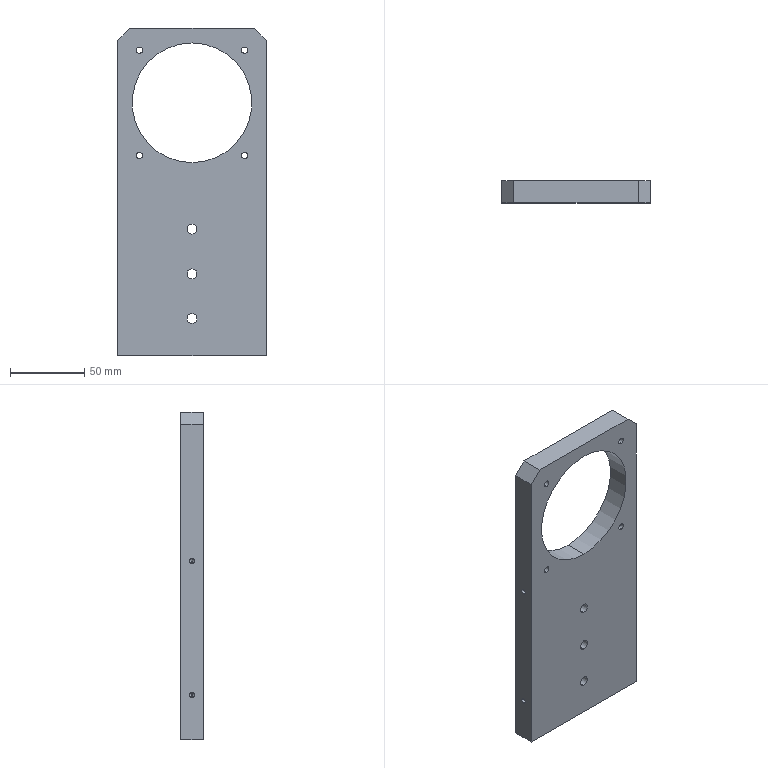Part | SolidWorks | features BaseBody 1 | 1 solid | 53 faces | box 100 x 15 x 220 mm | volume 247993 mm3 | cylinder 32 | plane 11 | cone 10 | commonest cylinder face diameters 4.2 x8 5 x6 6.6 x6 11 x6 3.3 x4 80.5 x2
STEP:
#1=CARTESIAN_POINT('',(-89.9,7.5,28.35));
#2=VERTEX_POINT('',#1);
#3=CARTESIAN_POINT('',(-89.9,7.5,31.65));
#4=VERTEX_POINT('',#3);
#5=CARTESIAN_POINT('',(-89.9,7.5,30.));
#6=DIRECTION('',(-1.,0.,0.));
#7=DIRECTION('',(0.,0.,1.));
#8=AXIS2_PLACEMENT_3D('',#5,#6,#7);
#9=CIRCLE('',#8,1.65);
#10=EDGE_CURVE('',#2,#4,#9,.T.);
#11=ORIENTED_EDGE('',*,*,#10,.F.);
#12=CARTESIAN_POINT('',(-100.,7.5,28.35));
#13=VERTEX_POINT('',#12);
#14=CARTESIAN_POINT('',(-100.,7.5,28.35));
#15=DIRECTION('',(-1.,0.,0.));
#16=VECTOR('',#15,1000.);
#17=LINE('',#14,#16);
#18=EDGE_CURVE('',#2,#13,#17,.T.);
#19=ORIENTED_EDGE('',*,*,#18,.T.);
#20=CARTESIAN_POINT('',(-100.,7.5,31.65));
#21=VERTEX_POINT('',#20);
#22=CARTESIAN_POINT('',(-100.,7.5,30.));
#23=DIRECTION('',(-1.,0.,0.));
#24=DIRECTION('',(0.,0.,1.));
#25=AXIS2_PLACEMENT_3D('',#22,#23,#24);
#26=CIRCLE('',#25,1.65);
#27=EDGE_CURVE('',#13,#21,#26,.T.);
#28=ORIENTED_EDGE('',*,*,#27,.T.);
#29=CARTESIAN_POINT('',(-100.,7.5,31.65));
#30=DIRECTION('',(-1.,0.,0.));
#31=VECTOR('',#30,1000.);
#32=LINE('',#29,#31);
#33=EDGE_CURVE('',#4,#21,#32,.T.);
#34=ORIENTED_EDGE('',*,*,#33,.F.);
#35=EDGE_LOOP('',(#11,#19,#28,#34));
#36=FACE_OUTER_BOUND('',#35,.T.);
#37=CARTESIAN_POINT('',(-100.,7.5,30.));
#38=DIRECTION('',(-1.,0.,0.));
#39=DIRECTION('',(0.,0.,1.));
#40=AXIS2_PLACEMENT_3D('',#37,#38,#39);
#41=CYLINDRICAL_SURFACE('',#40,1.65);
#42=ADVANCED_FACE('',(#36),#41,.F.);
#43=CARTESIAN_POINT('',(-88.909,7.5,30.));
#44=VERTEX_POINT('',#43);
#45=CARTESIAN_POINT('',(-89.9,7.5,31.65));
#46=DIRECTION('',(-0.515,0.,0.8572));
#47=VECTOR('',#46,1000.);
#48=LINE('',#45,#47);
#49=EDGE_CURVE('',#44,#4,#48,.T.);
#50=ORIENTED_EDGE('',*,*,#49,.F.);
#51=CARTESIAN_POINT('',(-89.9,7.5,28.35));
#52=DIRECTION('',(-0.515,0.,-0.8572));
#53=VECTOR('',#52,1000.);
#54=LINE('',#51,#53);
#55=EDGE_CURVE('',#44,#2,#54,.T.);
#56=ORIENTED_EDGE('',*,*,#55,.T.);
#57=ORIENTED_EDGE('',*,*,#10,.T.);
#58=EDGE_LOOP('',(#50,#56,#57));
#59=FACE_OUTER_BOUND('',#58,.T.);
#60=CARTESIAN_POINT('',(-89.9,7.5,30.));
#61=DIRECTION('',(-1.,0.,0.));
#62=DIRECTION('',(0.,0.,1.));
#63=AXIS2_PLACEMENT_3D('',#60,#61,#62);
#64=CONICAL_SURFACE('',#63,1.65,1.03);
#65=ADVANCED_FACE('',(#59),#64,.F.);
#66=CARTESIAN_POINT('',(-89.9,7.5,118.35));
#67=VERTEX_POINT('',#66);
#68=CARTESIAN_POINT('',(-89.9,7.5,121.65));
#69=VERTEX_POINT('',#68);
#70=CARTESIAN_POINT('',(-89.9,7.5,120.));
#71=DIRECTION('',(-1.,0.,0.));
#72=DIRECTION('',(0.,0.,1.));
#73=AXIS2_PLACEMENT_3D('',#70,#71,#72);
#74=CIRCLE('',#73,1.65);
#75=EDGE_CURVE('',#67,#69,#74,.T.);
#76=ORIENTED_EDGE('',*,*,#75,.F.);
#77=CARTESIAN_POINT('',(-100.,7.5,118.35));
#78=VERTEX_POINT('',#77);
#79=CARTESIAN_POINT('',(-100.,7.5,118.35));
#80=DIRECTION('',(-1.,0.,0.));
#81=VECTOR('',#80,1000.);
#82=LINE('',#79,#81);
#83=EDGE_CURVE('',#67,#78,#82,.T.);
#84=ORIENTED_EDGE('',*,*,#83,.T.);
#85=CARTESIAN_POINT('',(-100.,7.5,121.65));
#86=VERTEX_POINT('',#85);
#87=CARTESIAN_POINT('',(-100.,7.5,120.));
#88=DIRECTION('',(-1.,0.,0.));
#89=DIRECTION('',(0.,0.,1.));
#90=AXIS2_PLACEMENT_3D('',#87,#88,#89);
#91=CIRCLE('',#90,1.65);
#92=EDGE_CURVE('',#78,#86,#91,.T.);
#93=ORIENTED_EDGE('',*,*,#92,.T.);
#94=CARTESIAN_POINT('',(-100.,7.5,121.65));
#95=DIRECTION('',(-1.,0.,0.));
#96=VECTOR('',#95,1000.);
#97=LINE('',#94,#96);
#98=EDGE_CURVE('',#69,#86,#97,.T.);
#99=ORIENTED_EDGE('',*,*,#98,.F.);
#100=EDGE_LOOP('',(#76,#84,#93,#99));
#101=FACE_OUTER_BOUND('',#100,.T.);
#102=CARTESIAN_POINT('',(-100.,7.5,120.));
#103=DIRECTION('',(-1.,0.,0.));
#104=DIRECTION('',(0.,0.,1.));
#105=AXIS2_PLACEMENT_3D('',#102,#103,#104);
#106=CYLINDRICAL_SURFACE('',#105,1.65);
#107=ADVANCED_FACE('',(#101),#106,.F.);
#108=CARTESIAN_POINT('',(-88.909,7.5,120.));
#109=VERTEX_POINT('',#108);
#110=CARTESIAN_POINT('',(-89.9,7.5,121.65));
#111=DIRECTION('',(-0.515,0.,0.8572));
#112=VECTOR('',#111,1000.);
#113=LINE('',#110,#112);
#114=EDGE_CURVE('',#109,#69,#113,.T.);
#115=ORIENTED_EDGE('',*,*,#114,.F.);
#116=CARTESIAN_POINT('',(-89.9,7.5,118.35));
#117=DIRECTION('',(-0.515,0.,-0.8572));
#118=VECTOR('',#117,1000.);
#119=LINE('',#116,#118);
#120=EDGE_CURVE('',#109,#67,#119,.T.);
#121=ORIENTED_EDGE('',*,*,#120,.T.);
#122=ORIENTED_EDGE('',*,*,#75,.T.);
#123=EDGE_LOOP('',(#115,#121,#122));
#124=FACE_OUTER_BOUND('',#123,.T.);
#125=CARTESIAN_POINT('',(-89.9,7.5,120.));
#126=DIRECTION('',(-1.,0.,0.));
#127=DIRECTION('',(0.,0.,1.));
#128=AXIS2_PLACEMENT_3D('',#125,#126,#127);
#129=CONICAL_SURFACE('',#128,1.65,1.03);
#130=ADVANCED_FACE('',(#124),#129,.F.);
#131=CARTESIAN_POINT('',(-50.,8.2,19.5));
#132=VERTEX_POINT('',#131);
#133=CARTESIAN_POINT('',(-50.,8.2,30.5));
#134=VERTEX_POINT('',#133);
#135=CARTESIAN_POINT('',(-50.,8.2,25.));
#136=DIRECTION('',(0.,1.,0.));
#137=DIRECTION('',(0.,0.,1.));
#138=AXIS2_PLACEMENT_3D('',#135,#136,#137);
#139=CIRCLE('',#138,5.5);
#140=EDGE_CURVE('',#132,#134,#139,.T.);
#141=ORIENTED_EDGE('',*,*,#140,.F.);
#142=CARTESIAN_POINT('',(-50.,15.,19.5));
#143=VERTEX_POINT('',#142);
#144=CARTESIAN_POINT('',(-50.,15.,19.5));
#145=DIRECTION('',(0.,1.,0.));
#146=VECTOR('',#145,1000.);
#147=LINE('',#144,#146);
#148=EDGE_CURVE('',#132,#143,#147,.T.);
#149=ORIENTED_EDGE('',*,*,#148,.T.);
#150=CARTESIAN_POINT('',(-50.,15.,30.5));
#151=VERTEX_POINT('',#150);
#152=CARTESIAN_POINT('',(-50.,15.,25.));
#153=DIRECTION('',(0.,1.,0.));
#154=DIRECTION('',(0.,0.,1.));
#155=AXIS2_PLACEMENT_3D('',#152,#153,#154);
#156=CIRCLE('',#155,5.5);
#157=EDGE_CURVE('',#143,#151,#156,.T.);
#158=ORIENTED_EDGE('',*,*,#157,.T.);
#159=CARTESIAN_POINT('',(-50.,15.,30.5));
#160=DIRECTION('',(0.,1.,0.));
#161=VECTOR('',#160,1000.);
#162=LINE('',#159,#161);
#163=EDGE_CURVE('',#134,#151,#162,.T.);
#164=ORIENTED_EDGE('',*,*,#163,.F.);
#165=EDGE_LOOP('',(#141,#149,#158,#164));
#166=FACE_OUTER_BOUND('',#165,.T.);
#167=CARTESIAN_POINT('',(-50.,15.,25.));
#168=DIRECTION('',(0.,1.,0.));
#169=DIRECTION('',(0.,0.,1.));
#170=AXIS2_PLACEMENT_3D('',#167,#168,#169);
#171=CYLINDRICAL_SURFACE('',#170,5.5);
#172=ADVANCED_FACE('',(#166),#171,.F.);
#173=CARTESIAN_POINT('',(-50.,0.,21.7));
#174=VERTEX_POINT('',#173);
#175=CARTESIAN_POINT('',(-50.,0.,28.3));
#176=VERTEX_POINT('',#175);
#177=CARTESIAN_POINT('',(-50.,0.,25.));
#178=DIRECTION('',(0.,1.,0.));
#179=DIRECTION('',(0.,0.,1.));
#180=AXIS2_PLACEMENT_3D('',#177,#178,#179);
#181=CIRCLE('',#180,3.3);
#182=EDGE_CURVE('',#174,#176,#181,.T.);
#183=ORIENTED_EDGE('',*,*,#182,.F.);
#184=CARTESIAN_POINT('',(-50.,8.2,21.7));
#185=VERTEX_POINT('',#184);
#186=CARTESIAN_POINT('',(-50.,15.,21.7));
#187=DIRECTION('',(0.,1.,0.));
#188=VECTOR('',#187,1000.);
#189=LINE('',#186,#188);
#190=EDGE_CURVE('',#174,#185,#189,.T.);
#191=ORIENTED_EDGE('',*,*,#190,.T.);
#192=CARTESIAN_POINT('',(-50.,8.2,28.3));
#193=VERTEX_POINT('',#192);
#194=CARTESIAN_POINT('',(-50.,8.2,25.));
#195=DIRECTION('',(0.,1.,0.));
#196=DIRECTION('',(0.,0.,1.));
#197=AXIS2_PLACEMENT_3D('',#194,#195,#196);
#198=CIRCLE('',#197,3.3);
#199=EDGE_CURVE('',#185,#193,#198,.T.);
#200=ORIENTED_EDGE('',*,*,#199,.T.);
#201=CARTESIAN_POINT('',(-50.,15.,28.3));
#202=DIRECTION('',(0.,1.,0.));
#203=VECTOR('',#202,1000.);
#204=LINE('',#201,#203);
#205=EDGE_CURVE('',#176,#193,#204,.T.);
#206=ORIENTED_EDGE('',*,*,#205,.F.);
#207=EDGE_LOOP('',(#183,#191,#200,#206));
#208=FACE_OUTER_BOUND('',#207,.T.);
#209=CARTESIAN_POINT('',(-50.,15.,25.));
#210=DIRECTION('',(0.,1.,0.));
#211=DIRECTION('',(0.,0.,1.));
#212=AXIS2_PLACEMENT_3D('',#209,#210,#211);
#213=CYLINDRICAL_SURFACE('',#212,3.3);
#214=ADVANCED_FACE('',(#208),#213,.F.);
#215=CARTESIAN_POINT('',(-50.,8.2,79.5));
#216=VERTEX_POINT('',#215);
#217=CARTESIAN_POINT('',(-50.,8.2,90.5));
#218=VERTEX_POINT('',#217);
#219=CARTESIAN_POINT('',(-50.,8.2,85.));
#220=DIRECTION('',(0.,1.,0.));
#221=DIRECTION('',(0.,0.,1.));
#222=AXIS2_PLACEMENT_3D('',#219,#220,#221);
#223=CIRCLE('',#222,5.5);
#224=EDGE_CURVE('',#216,#218,#223,.T.);
#225=ORIENTED_EDGE('',*,*,#224,.F.);
#226=CARTESIAN_POINT('',(-50.,15.,79.5));
#227=VERTEX_POINT('',#226);
#228=CARTESIAN_POINT('',(-50.,15.,79.5));
#229=DIRECTION('',(0.,1.,0.));
#230=VECTOR('',#229,1000.);
#231=LINE('',#228,#230);
#232=EDGE_CURVE('',#216,#227,#231,.T.);
#233=ORIENTED_EDGE('',*,*,#232,.T.);
#234=CARTESIAN_POINT('',(-50.,15.,90.5));
#235=VERTEX_POINT('',#234);
#236=CARTESIAN_POINT('',(-50.,15.,85.));
#237=DIRECTION('',(0.,1.,0.));
#238=DIRECTION('',(0.,0.,1.));
#239=AXIS2_PLACEMENT_3D('',#236,#237,#238);
#240=CIRCLE('',#239,5.5);
#241=EDGE_CURVE('',#227,#235,#240,.T.);
#242=ORIENTED_EDGE('',*,*,#241,.T.);
#243=CARTESIAN_POINT('',(-50.,15.,90.5));
#244=DIRECTION('',(0.,1.,0.));
#245=VECTOR('',#244,1000.);
#246=LINE('',#243,#245);
#247=EDGE_CURVE('',#218,#235,#246,.T.);
#248=ORIENTED_EDGE('',*,*,#247,.F.);
#249=EDGE_LOOP('',(#225,#233,#242,#248));
#250=FACE_OUTER_BOUND('',#249,.T.);
#251=CARTESIAN_POINT('',(-50.,15.,85.));
#252=DIRECTION('',(0.,1.,0.));
#253=DIRECTION('',(0.,0.,1.));
#254=AXIS2_PLACEMENT_3D('',#251,#252,#253);
#255=CYLINDRICAL_SURFACE('',#254,5.5);
#256=ADVANCED_FACE('',(#250),#255,.F.);
#257=CARTESIAN_POINT('',(-50.,0.,81.7));
#258=VERTEX_POINT('',#257);
#259=CARTESIAN_POINT('',(-50.,0.,88.3));
#260=VERTEX_POINT('',#259);
#261=CARTESIAN_POINT('',(-50.,0.,85.));
#262=DIRECTION('',(0.,1.,0.));
#263=DIRECTION('',(0.,0.,1.));
#264=AXIS2_PLACEMENT_3D('',#261,#262,#263);
#265=CIRCLE('',#264,3.3);
#266=EDGE_CURVE('',#258,#260,#265,.T.);
#267=ORIENTED_EDGE('',*,*,#266,.F.);
#268=CARTESIAN_POINT('',(-50.,8.2,81.7));
#269=VERTEX_POINT('',#268);
#270=CARTESIAN_POINT('',(-50.,15.,81.7));
#271=DIRECTION('',(0.,1.,0.));
#272=VECTOR('',#271,1000.);
#273=LINE('',#270,#272);
#274=EDGE_CURVE('',#258,#269,#273,.T.);
#275=ORIENTED_EDGE('',*,*,#274,.T.);
#276=CARTESIAN_POINT('',(-50.,8.2,88.3));
#277=VERTEX_POINT('',#276);
#278=CARTESIAN_POINT('',(-50.,8.2,85.));
#279=DIRECTION('',(0.,1.,0.));
#280=DIRECTION('',(0.,0.,1.));
#281=AXIS2_PLACEMENT_3D('',#278,#279,#280);
#282=CIRCLE('',#281,3.3);
#283=EDGE_CURVE('',#269,#277,#282,.T.);
#284=ORIENTED_EDGE('',*,*,#283,.T.);
#285=CARTESIAN_POINT('',(-50.,15.,88.3));
#286=DIRECTION('',(0.,1.,0.));
#287=VECTOR('',#286,1000.);
#288=LINE('',#285,#287);
#289=EDGE_CURVE('',#260,#277,#288,.T.);
#290=ORIENTED_EDGE('',*,*,#289,.F.);
#291=EDGE_LOOP('',(#267,#275,#284,#290));
#292=FACE_OUTER_BOUND('',#291,.T.);
#293=CARTESIAN_POINT('',(-50.,15.,85.));
#294=DIRECTION('',(0.,1.,0.));
#295=DIRECTION('',(0.,0.,1.));
#296=AXIS2_PLACEMENT_3D('',#293,#294,#295);
#297=CYLINDRICAL_SURFACE('',#296,3.3);
#298=ADVANCED_FACE('',(#292),#297,.F.);
#299=CARTESIAN_POINT('',(-50.,8.2,49.5));
#300=VERTEX_POINT('',#299);
#301=CARTESIAN_POINT('',(-50.,8.2,60.5));
#302=VERTEX_POINT('',#301);
#303=CARTESIAN_POINT('',(-50.,8.2,55.));
#304=DIRECTION('',(0.,1.,0.));
#305=DIRECTION('',(0.,0.,1.));
#306=AXIS2_PLACEMENT_3D('',#303,#304,#305);
#307=CIRCLE('',#306,5.5);
#308=EDGE_CURVE('',#300,#302,#307,.T.);
#309=ORIENTED_EDGE('',*,*,#308,.F.);
#310=CARTESIAN_POINT('',(-50.,15.,49.5));
#311=VERTEX_POINT('',#310);
#312=CARTESIAN_POINT('',(-50.,15.,49.5));
#313=DIRECTION('',(0.,1.,0.));
#314=VECTOR('',#313,1000.);
#315=LINE('',#312,#314);
#316=EDGE_CURVE('',#300,#311,#315,.T.);
#317=ORIENTED_EDGE('',*,*,#316,.T.);
#318=CARTESIAN_POINT('',(-50.,15.,60.5));
#319=VERTEX_POINT('',#318);
#320=CARTESIAN_POINT('',(-50.,15.,55.));
#321=DIRECTION('',(0.,1.,0.));
#322=DIRECTION('',(0.,0.,1.));
#323=AXIS2_PLACEMENT_3D('',#320,#321,#322);
#324=CIRCLE('',#323,5.5);
#325=EDGE_CURVE('',#311,#319,#324,.T.);
#326=ORIENTED_EDGE('',*,*,#325,.T.);
#327=CARTESIAN_POINT('',(-50.,15.,60.5));
#328=DIRECTION('',(0.,1.,0.));
#329=VECTOR('',#328,1000.);
#330=LINE('',#327,#329);
#331=EDGE_CURVE('',#302,#319,#330,.T.);
#332=ORIENTED_EDGE('',*,*,#331,.F.);
#333=EDGE_LOOP('',(#309,#317,#326,#332));
#334=FACE_OUTER_BOUND('',#333,.T.);
#335=CARTESIAN_POINT('',(-50.,15.,55.));
#336=DIRECTION('',(0.,1.,0.));
#337=DIRECTION('',(0.,0.,1.));
#338=AXIS2_PLACEMENT_3D('',#335,#336,#337);
#339=CYLINDRICAL_SURFACE('',#338,5.5);
#340=ADVANCED_FACE('',(#334),#339,.F.);
#341=CARTESIAN_POINT('',(-50.,0.,51.7));
#342=VERTEX_POINT('',#341);
#343=CARTESIAN_POINT('',(-50.,0.,58.3));
#344=VERTEX_POINT('',#343);
#345=CARTESIAN_POINT('',(-50.,0.,55.));
#346=DIRECTION('',(0.,1.,0.));
#347=DIRECTION('',(0.,0.,1.));
#348=AXIS2_PLACEMENT_3D('',#345,#346,#347);
#349=CIRCLE('',#348,3.3);
#350=EDGE_CURVE('',#342,#344,#349,.T.);
#351=ORIENTED_EDGE('',*,*,#350,.F.);
#352=CARTESIAN_POINT('',(-50.,8.2,51.7));
#353=VERTEX_POINT('',#352);
#354=CARTESIAN_POINT('',(-50.,15.,51.7));
#355=DIRECTION('',(0.,1.,0.));
#356=VECTOR('',#355,1000.);
#357=LINE('',#354,#356);
#358=EDGE_CURVE('',#342,#353,#357,.T.);
#359=ORIENTED_EDGE('',*,*,#358,.T.);
#360=CARTESIAN_POINT('',(-50.,8.2,58.3));
#361=VERTEX_POINT('',#360);
#362=CARTESIAN_POINT('',(-50.,8.2,55.));
#363=DIRECTION('',(0.,1.,0.));
#364=DIRECTION('',(0.,0.,1.));
#365=AXIS2_PLACEMENT_3D('',#362,#363,#364);
#366=CIRCLE('',#365,3.3);
#367=EDGE_CURVE('',#353,#361,#366,.T.);
#368=ORIENTED_EDGE('',*,*,#367,.T.);
#369=CARTESIAN_POINT('',(-50.,15.,58.3));
#370=DIRECTION('',(0.,1.,0.));
#371=VECTOR('',#370,1000.);
#372=LINE('',#369,#371);
#373=EDGE_CURVE('',#344,#361,#372,.T.);
#374=ORIENTED_EDGE('',*,*,#373,.F.);
#375=EDGE_LOOP('',(#351,#359,#368,#374));
#376=FACE_OUTER_BOUND('',#375,.T.);
#377=CARTESIAN_POINT('',(-50.,15.,55.));
#378=DIRECTION('',(0.,1.,0.));
#379=DIRECTION('',(0.,0.,1.));
#380=AXIS2_PLACEMENT_3D('',#377,#378,#379);
#381=CYLINDRICAL_SURFACE('',#380,3.3);
#382=ADVANCED_FACE('',(#376),#381,.F.);
#383=CARTESIAN_POINT('',(-47.5,7.5,15.));
#384=VERTEX_POINT('',#383);
#385=CARTESIAN_POINT('',(-52.5,7.5,15.));
#386=VERTEX_POINT('',#385);
#387=CARTESIAN_POINT('',(-50.,7.5,15.));
#388=DIRECTION('',(0.,0.,-1.));
#389=DIRECTION('',(-1.,0.,0.));
#390=AXIS2_PLACEMENT_3D('',#387,#388,#389);
#391=CIRCLE('',#390,2.5);
#392=EDGE_CURVE('',#384,#386,#391,.T.);
#393=ORIENTED_EDGE('',*,*,#392,.F.);
#394=CARTESIAN_POINT('',(-47.5,7.5,0.));
#395=VERTEX_POINT('',#394);
#396=CARTESIAN_POINT('',(-47.5,7.5,0.));
#397=DIRECTION('',(0.,0.,-1.));
#398=VECTOR('',#397,1000.);
#399=LINE('',#396,#398);
#400=EDGE_CURVE('',#384,#395,#399,.T.);
#401=ORIENTED_EDGE('',*,*,#400,.T.);
#402=CARTESIAN_POINT('',(-52.5,7.5,0.));
#403=VERTEX_POINT('',#402);
#404=CARTESIAN_POINT('',(-50.,7.5,0.));
#405=DIRECTION('',(0.,0.,-1.));
#406=DIRECTION('',(-1.,0.,0.));
#407=AXIS2_PLACEMENT_3D('',#404,#405,#406);
#408=CIRCLE('',#407,2.5);
#409=EDGE_CURVE('',#395,#403,#408,.T.);
#410=ORIENTED_EDGE('',*,*,#409,.T.);
#411=CARTESIAN_POINT('',(-52.5,7.5,0.));
#412=DIRECTION('',(0.,0.,-1.));
#413=VECTOR('',#412,1000.);
#414=LINE('',#411,#413);
#415=EDGE_CURVE('',#386,#403,#414,.T.);
#416=ORIENTED_EDGE('',*,*,#415,.F.);
#417=EDGE_LOOP('',(#393,#401,#410,#416));
#418=FACE_OUTER_BOUND('',#417,.T.);
#419=CARTESIAN_POINT('',(-50.,7.5,0.));
#420=DIRECTION('',(0.,0.,-1.));
#421=DIRECTION('',(-1.,0.,0.));
#422=AXIS2_PLACEMENT_3D('',#419,#420,#421);
#423=CYLINDRICAL_SURFACE('',#422,2.5);
#424=ADVANCED_FACE('',(#418),#423,.F.);
#425=CARTESIAN_POINT('',(-50.,7.5,16.502));
#426=VERTEX_POINT('',#425);
#427=CARTESIAN_POINT('',(-52.5,7.5,15.));
#428=DIRECTION('',(-0.8572,0.,-0.515));
#429=VECTOR('',#428,1000.);
#430=LINE('',#427,#429);
#431=EDGE_CURVE('',#426,#386,#430,.T.);
#432=ORIENTED_EDGE('',*,*,#431,.F.);
#433=CARTESIAN_POINT('',(-47.5,7.5,15.));
#434=DIRECTION('',(0.8572,0.,-0.515));
#435=VECTOR('',#434,1000.);
#436=LINE('',#433,#435);
#437=EDGE_CURVE('',#426,#384,#436,.T.);
#438=ORIENTED_EDGE('',*,*,#437,.T.);
#439=ORIENTED_EDGE('',*,*,#392,.T.);
#440=EDGE_LOOP('',(#432,#438,#439));
#441=FACE_OUTER_BOUND('',#440,.T.);
#442=CARTESIAN_POINT('',(-50.,7.5,15.));
#443=DIRECTION('',(0.,0.,-1.));
#444=DIRECTION('',(-1.,0.,0.));
#445=AXIS2_PLACEMENT_3D('',#442,#443,#444);
#446=CONICAL_SURFACE('',#445,2.5,1.03);
#447=ADVANCED_FACE('',(#441),#446,.F.);
#448=CARTESIAN_POINT('',(-7.5,7.5,15.));
#449=VERTEX_POINT('',#448);
#450=CARTESIAN_POINT('',(-12.5,7.5,15.));
#451=VERTEX_POINT('',#450);
#452=CARTESIAN_POINT('',(-10.,7.5,15.));
#453=DIRECTION('',(0.,0.,-1.));
#454=DIRECTION('',(-1.,0.,0.));
#455=AXIS2_PLACEMENT_3D('',#452,#453,#454);
#456=CIRCLE('',#455,2.5);
#457=EDGE_CURVE('',#449,#451,#456,.T.);
#458=ORIENTED_EDGE('',*,*,#457,.F.);
#459=CARTESIAN_POINT('',(-7.5,7.5,0.));
#460=VERTEX_POINT('',#459);
#461=CARTESIAN_POINT('',(-7.5,7.5,0.));
#462=DIRECTION('',(0.,0.,-1.));
#463=VECTOR('',#462,1000.);
#464=LINE('',#461,#463);
#465=EDGE_CURVE('',#449,#460,#464,.T.);
#466=ORIENTED_EDGE('',*,*,#465,.T.);
#467=CARTESIAN_POINT('',(-12.5,7.5,0.));
#468=VERTEX_POINT('',#467);
#469=CARTESIAN_POINT('',(-10.,7.5,0.));
#470=DIRECTION('',(0.,0.,-1.));
#471=DIRECTION('',(-1.,0.,0.));
#472=AXIS2_PLACEMENT_3D('',#469,#470,#471);
#473=CIRCLE('',#472,2.5);
#474=EDGE_CURVE('',#460,#468,#473,.T.);
#475=ORIENTED_EDGE('',*,*,#474,.T.);
#476=CARTESIAN_POINT('',(-12.5,7.5,0.));
#477=DIRECTION('',(0.,0.,-1.));
#478=VECTOR('',#477,1000.);
#479=LINE('',#476,#478);
#480=EDGE_CURVE('',#451,#468,#479,.T.);
#481=ORIENTED_EDGE('',*,*,#480,.F.);
#482=EDGE_LOOP('',(#458,#466,#475,#481));
#483=FACE_OUTER_BOUND('',#482,.T.);
#484=CARTESIAN_POINT('',(-10.,7.5,0.));
#485=DIRECTION('',(0.,0.,-1.));
#486=DIRECTION('',(-1.,0.,0.));
#487=AXIS2_PLACEMENT_3D('',#484,#485,#486);
#488=CYLINDRICAL_SURFACE('',#487,2.5);
#489=ADVANCED_FACE('',(#483),#488,.F.);
#490=CARTESIAN_POINT('',(-10.,7.5,16.502));
#491=VERTEX_POINT('',#490);
#492=CARTESIAN_POINT('',(-12.5,7.5,15.));
#493=DIRECTION('',(-0.8572,0.,-0.515));
#494=VECTOR('',#493,1000.);
#495=LINE('',#492,#494);
#496=EDGE_CURVE('',#491,#451,#495,.T.);
#497=ORIENTED_EDGE('',*,*,#496,.F.);
#498=CARTESIAN_POINT('',(-7.5,7.5,15.));
#499=DIRECTION('',(0.8572,0.,-0.515));
#500=VECTOR('',#499,1000.);
#501=LINE('',#498,#500);
#502=EDGE_CURVE('',#491,#449,#501,.T.);
#503=ORIENTED_EDGE('',*,*,#502,.T.);
#504=ORIENTED_EDGE('',*,*,#457,.T.);
#505=EDGE_LOOP('',(#497,#503,#504));
#506=FACE_OUTER_BOUND('',#505,.T.);
#507=CARTESIAN_POINT('',(-10.,7.5,15.));
#508=DIRECTION('',(0.,0.,-1.));
#509=DIRECTION('',(-1.,0.,0.));
#510=AXIS2_PLACEMENT_3D('',#507,#508,#509);
#511=CONICAL_SURFACE('',#510,2.5,1.03);
#512=ADVANCED_FACE('',(#506),#511,.F.);
#513=CARTESIAN_POINT('',(-87.5,7.5,15.));
#514=VERTEX_POINT('',#513);
#515=CARTESIAN_POINT('',(-92.5,7.5,15.));
#516=VERTEX_POINT('',#515);
#517=CARTESIAN_POINT('',(-90.,7.5,15.));
#518=DIRECTION('',(0.,0.,-1.));
#519=DIRECTION('',(-1.,0.,0.));
#520=AXIS2_PLACEMENT_3D('',#517,#518,#519);
#521=CIRCLE('',#520,2.5);
#522=EDGE_CURVE('',#514,#516,#521,.T.);
#523=ORIENTED_EDGE('',*,*,#522,.F.);
#524=CARTESIAN_POINT('',(-87.5,7.5,0.));
#525=VERTEX_POINT('',#524);
#526=CARTESIAN_POINT('',(-87.5,7.5,0.));
#527=DIRECTION('',(0.,0.,-1.));
#528=VECTOR('',#527,1000.);
#529=LINE('',#526,#528);
#530=EDGE_CURVE('',#514,#525,#529,.T.);
#531=ORIENTED_EDGE('',*,*,#530,.T.);
#532=CARTESIAN_POINT('',(-92.5,7.5,0.));
#533=VERTEX_POINT('',#532);
#534=CARTESIAN_POINT('',(-90.,7.5,0.));
#535=DIRECTION('',(0.,0.,-1.));
#536=DIRECTION('',(-1.,0.,0.));
#537=AXIS2_PLACEMENT_3D('',#534,#535,#536);
#538=CIRCLE('',#537,2.5);
#539=EDGE_CURVE('',#525,#533,#538,.T.);
#540=ORIENTED_EDGE('',*,*,#539,.T.);
#541=CARTESIAN_POINT('',(-92.5,7.5,0.));
#542=DIRECTION('',(0.,0.,-1.));
#543=VECTOR('',#542,1000.);
#544=LINE('',#541,#543);
#545=EDGE_CURVE('',#516,#533,#544,.T.);
#546=ORIENTED_EDGE('',*,*,#545,.F.);
#547=EDGE_LOOP('',(#523,#531,#540,#546));
#548=FACE_OUTER_BOUND('',#547,.T.);
#549=CARTESIAN_POINT('',(-90.,7.5,0.));
#550=DIRECTION('',(0.,0.,-1.));
#551=DIRECTION('',(-1.,0.,0.));
#552=AXIS2_PLACEMENT_3D('',#549,#550,#551);
#553=CYLINDRICAL_SURFACE('',#552,2.5);
#554=ADVANCED_FACE('',(#548),#553,.F.);
#555=CARTESIAN_POINT('',(-90.,7.5,16.502));
#556=VERTEX_POINT('',#555);
#557=CARTESIAN_POINT('',(-92.5,7.5,15.));
#558=DIRECTION('',(-0.8572,0.,-0.515));
#559=VECTOR('',#558,1000.);
#560=LINE('',#557,#559);
#561=EDGE_CURVE('',#556,#516,#560,.T.);
#562=ORIENTED_EDGE('',*,*,#561,.F.);
#563=CARTESIAN_POINT('',(-87.5,7.5,15.));
#564=DIRECTION('',(0.8572,0.,-0.515));
#565=VECTOR('',#564,1000.);
#566=LINE('',#563,#565);
#567=EDGE_CURVE('',#556,#514,#566,.T.);
#568=ORIENTED_EDGE('',*,*,#567,.T.);
#569=ORIENTED_EDGE('',*,*,#522,.T.);
#570=EDGE_LOOP('',(#562,#568,#569));
#571=FACE_OUTER_BOUND('',#570,.T.);
#572=CARTESIAN_POINT('',(-90.,7.5,15.));
#573=DIRECTION('',(0.,0.,-1.));
#574=DIRECTION('',(-1.,0.,0.));
#575=AXIS2_PLACEMENT_3D('',#572,#573,#574);
#576=CONICAL_SURFACE('',#575,2.5,1.03);
#577=ADVANCED_FACE('',(#571),#576,.F.);
#578=CARTESIAN_POINT('',(-85.355,15.,203.255));
#579=VERTEX_POINT('',#578);
#580=CARTESIAN_POINT('',(-85.355,15.,207.455));
#581=VERTEX_POINT('',#580);
#582=CARTESIAN_POINT('',(-85.355,15.,205.355));
#583=DIRECTION('',(0.,1.,0.));
#584=DIRECTION('',(0.,0.,1.));
#585=AXIS2_PLACEMENT_3D('',#582,#583,#584);
#586=CIRCLE('',#585,2.1);
#587=EDGE_CURVE('',#579,#581,#586,.T.);
#588=ORIENTED_EDGE('',*,*,#587,.T.);
#589=CARTESIAN_POINT('',(-85.355,0.,207.455));
#590=VERTEX_POINT('',#589);
#591=CARTESIAN_POINT('',(-85.355,0.,207.455));
#592=DIRECTION('',(0.,-1.,0.));
#593=VECTOR('',#592,1000.);
#594=LINE('',#591,#593);
#595=EDGE_CURVE('',#581,#590,#594,.T.);
#596=ORIENTED_EDGE('',*,*,#595,.T.);
#597=CARTESIAN_POINT('',(-85.355,0.,203.255));
#598=VERTEX_POINT('',#597);
#599=CARTESIAN_POINT('',(-85.355,0.,205.355));
#600=DIRECTION('',(0.,-1.,0.));
#601=DIRECTION('',(0.,0.,-1.));
#602=AXIS2_PLACEMENT_3D('',#599,#600,#601);
#603=CIRCLE('',#602,2.1);
#604=EDGE_CURVE('',#590,#598,#603,.T.);
#605=ORIENTED_EDGE('',*,*,#604,.T.);
#606=CARTESIAN_POINT('',(-85.355,0.,203.255));
#607=DIRECTION('',(0.,-1.,0.));
#608=VECTOR('',#607,1000.);
#609=LINE('',#606,#608);
#610=EDGE_CURVE('',#579,#598,#609,.T.);
#611=ORIENTED_EDGE('',*,*,#610,.F.);
#612=EDGE_LOOP('',(#588,#596,#605,#611));
#613=FACE_OUTER_BOUND('',#612,.T.);
#614=CARTESIAN_POINT('',(-85.355,0.,205.355));
#615=DIRECTION('',(0.,-1.,0.));
#616=DIRECTION('',(0.,0.,-1.));
#617=AXIS2_PLACEMENT_3D('',#614,#615,#616);
#618=CYLINDRICAL_SURFACE('',#617,2.1);
#619=ADVANCED_FACE('',(#613),#618,.F.);
#620=CARTESIAN_POINT('',(-14.645,15.,132.545));
#621=VERTEX_POINT('',#620);
#622=CARTESIAN_POINT('',(-14.645,15.,136.745));
#623=VERTEX_POINT('',#622);
#624=CARTESIAN_POINT('',(-14.645,15.,134.645));
#625=DIRECTION('',(0.,1.,0.));
#626=DIRECTION('',(0.,0.,1.));
#627=AXIS2_PLACEMENT_3D('',#624,#625,#626);
#628=CIRCLE('',#627,2.1);
#629=EDGE_CURVE('',#621,#623,#628,.T.);
#630=ORIENTED_EDGE('',*,*,#629,.T.);
#631=CARTESIAN_POINT('',(-14.645,0.,136.745));
#632=VERTEX_POINT('',#631);
#633=CARTESIAN_POINT('',(-14.645,0.,136.745));
#634=DIRECTION('',(0.,-1.,0.));
#635=VECTOR('',#634,1000.);
#636=LINE('',#633,#635);
#637=EDGE_CURVE('',#623,#632,#636,.T.);
#638=ORIENTED_EDGE('',*,*,#637,.T.);
#639=CARTESIAN_POINT('',(-14.645,0.,132.545));
#640=VERTEX_POINT('',#639);
#641=CARTESIAN_POINT('',(-14.645,0.,134.645));
#642=DIRECTION('',(0.,-1.,0.));
#643=DIRECTION('',(0.,0.,-1.));
#644=AXIS2_PLACEMENT_3D('',#641,#642,#643);
#645=CIRCLE('',#644,2.1);
#646=EDGE_CURVE('',#632,#640,#645,.T.);
#647=ORIENTED_EDGE('',*,*,#646,.T.);
#648=CARTESIAN_POINT('',(-14.645,0.,132.545));
#649=DIRECTION('',(0.,-1.,0.));
#650=VECTOR('',#649,1000.);
#651=LINE('',#648,#650);
#652=EDGE_CURVE('',#621,#640,#651,.T.);
#653=ORIENTED_EDGE('',*,*,#652,.F.);
#654=EDGE_LOOP('',(#630,#638,#647,#653));
#655=FACE_OUTER_BOUND('',#654,.T.);
#656=CARTESIAN_POINT('',(-14.645,0.,134.645));
#657=DIRECTION('',(0.,-1.,0.));
#658=DIRECTION('',(0.,0.,-1.));
#659=AXIS2_PLACEMENT_3D('',#656,#657,#658);
#660=CYLINDRICAL_SURFACE('',#659,2.1);
#661=ADVANCED_FACE('',(#655),#660,.F.);
#662=CARTESIAN_POINT('',(-85.355,15.,132.545));
#663=VERTEX_POINT('',#662);
#664=CARTESIAN_POINT('',(-85.355,15.,136.745));
#665=VERTEX_POINT('',#664);
#666=CARTESIAN_POINT('',(-85.355,15.,134.645));
#667=DIRECTION('',(0.,1.,0.));
#668=DIRECTION('',(0.,0.,1.));
#669=AXIS2_PLACEMENT_3D('',#666,#667,#668);
#670=CIRCLE('',#669,2.1);
#671=EDGE_CURVE('',#663,#665,#670,.T.);
#672=ORIENTED_EDGE('',*,*,#671,.T.);
#673=CARTESIAN_POINT('',(-85.355,0.,136.745));
#674=VERTEX_POINT('',#673);
#675=CARTESIAN_POINT('',(-85.355,0.,136.745));
#676=DIRECTION('',(0.,-1.,0.));
#677=VECTOR('',#676,1000.);
#678=LINE('',#675,#677);
#679=EDGE_CURVE('',#665,#674,#678,.T.);
#680=ORIENTED_EDGE('',*,*,#679,.T.);
#681=CARTESIAN_POINT('',(-85.355,0.,132.545));
#682=VERTEX_POINT('',#681);
#683=CARTESIAN_POINT('',(-85.355,0.,134.645));
#684=DIRECTION('',(0.,-1.,0.));
#685=DIRECTION('',(0.,0.,-1.));
#686=AXIS2_PLACEMENT_3D('',#683,#684,#685);
#687=CIRCLE('',#686,2.1);
#688=EDGE_CURVE('',#674,#682,#687,.T.);
#689=ORIENTED_EDGE('',*,*,#688,.T.);
#690=CARTESIAN_POINT('',(-85.355,0.,132.545));
#691=DIRECTION('',(0.,-1.,0.));
#692=VECTOR('',#691,1000.);
#693=LINE('',#690,#692);
#694=EDGE_CURVE('',#663,#682,#693,.T.);
#695=ORIENTED_EDGE('',*,*,#694,.F.);
#696=EDGE_LOOP('',(#672,#680,#689,#695));
#697=FACE_OUTER_BOUND('',#696,.T.);
#698=CARTESIAN_POINT('',(-85.355,0.,134.645));
#699=DIRECTION('',(0.,-1.,0.));
#700=DIRECTION('',(0.,0.,-1.));
#701=AXIS2_PLACEMENT_3D('',#698,#699,#700);
#702=CYLINDRICAL_SURFACE('',#701,2.1);
#703=ADVANCED_FACE('',(#697),#702,.F.);
#704=CARTESIAN_POINT('',(-14.645,15.,203.255));
#705=VERTEX_POINT('',#704);
#706=CARTESIAN_POINT('',(-14.645,15.,207.455));
#707=VERTEX_POINT('',#706);
#708=CARTESIAN_POINT('',(-14.645,15.,205.355));
#709=DIRECTION('',(0.,1.,0.));
#710=DIRECTION('',(0.,0.,1.));
#711=AXIS2_PLACEMENT_3D('',#708,#709,#710);
#712=CIRCLE('',#711,2.1);
#713=EDGE_CURVE('',#705,#707,#712,.T.);
#714=ORIENTED_EDGE('',*,*,#713,.T.);
#715=CARTESIAN_POINT('',(-14.645,0.,207.455));
#716=VERTEX_POINT('',#715);
#717=CARTESIAN_POINT('',(-14.645,0.,207.455));
#718=DIRECTION('',(0.,-1.,0.));
#719=VECTOR('',#718,1000.);
#720=LINE('',#717,#719);
#721=EDGE_CURVE('',#707,#716,#720,.T.);
#722=ORIENTED_EDGE('',*,*,#721,.T.);
#723=CARTESIAN_POINT('',(-14.645,0.,203.255));
#724=VERTEX_POINT('',#723);
#725=CARTESIAN_POINT('',(-14.645,0.,205.355));
#726=DIRECTION('',(0.,-1.,0.));
#727=DIRECTION('',(0.,0.,-1.));
#728=AXIS2_PLACEMENT_3D('',#725,#726,#727);
#729=CIRCLE('',#728,2.1);
#730=EDGE_CURVE('',#716,#724,#729,.T.);
#731=ORIENTED_EDGE('',*,*,#730,.T.);
#732=CARTESIAN_POINT('',(-14.645,0.,203.255));
#733=DIRECTION('',(0.,-1.,0.));
#734=VECTOR('',#733,1000.);
#735=LINE('',#732,#734);
#736=EDGE_CURVE('',#705,#724,#735,.T.);
#737=ORIENTED_EDGE('',*,*,#736,.F.);
#738=EDGE_LOOP('',(#714,#722,#731,#737));
#739=FACE_OUTER_BOUND('',#738,.T.);
#740=CARTESIAN_POINT('',(-14.645,0.,205.355));
#741=DIRECTION('',(0.,-1.,0.));
#742=DIRECTION('',(0.,0.,-1.));
#743=AXIS2_PLACEMENT_3D('',#740,#741,#742);
#744=CYLINDRICAL_SURFACE('',#743,2.1);
#745=ADVANCED_FACE('',(#739),#744,.F.);
#746=CARTESIAN_POINT('',(-50.,15.,129.75));
#747=VERTEX_POINT('',#746);
#748=CARTESIAN_POINT('',(-50.,15.,210.25));
#749=VERTEX_POINT('',#748);
#750=CARTESIAN_POINT('',(-50.,15.,170.));
#751=DIRECTION('',(0.,1.,0.));
#752=DIRECTION('',(0.,0.,1.));
#753=AXIS2_PLACEMENT_3D('',#750,#751,#752);
#754=CIRCLE('',#753,40.25);
#755=EDGE_CURVE('',#747,#749,#754,.T.);
#756=ORIENTED_EDGE('',*,*,#755,.T.);
#757=CARTESIAN_POINT('',(-50.,0.,210.25));
#758=VERTEX_POINT('',#757);
#759=CARTESIAN_POINT('',(-50.,15.,210.25));
#760=DIRECTION('',(0.,-1.,0.));
#761=VECTOR('',#760,1000.);
#762=LINE('',#759,#761);
#763=EDGE_CURVE('',#749,#758,#762,.T.);
#764=ORIENTED_EDGE('',*,*,#763,.T.);
#765=CARTESIAN_POINT('',(-50.,0.,129.75));
#766=VERTEX_POINT('',#765);
#767=CARTESIAN_POINT('',(-50.,0.,170.));
#768=DIRECTION('',(0.,1.,0.));
#769=DIRECTION('',(0.,0.,1.));
#770=AXIS2_PLACEMENT_3D('',#767,#768,#769);
#771=CIRCLE('',#770,40.25);
#772=EDGE_CURVE('',#766,#758,#771,.T.);
#773=ORIENTED_EDGE('',*,*,#772,.F.);
#774=CARTESIAN_POINT('',(-50.,15.,129.75));
#775=DIRECTION('',(0.,-1.,0.));
#776=VECTOR('',#775,1000.);
#777=LINE('',#774,#776);
#778=EDGE_CURVE('',#747,#766,#777,.T.);
#779=ORIENTED_EDGE('',*,*,#778,.F.);
#780=EDGE_LOOP('',(#756,#764,#773,#779));
#781=FACE_OUTER_BOUND('',#780,.T.);
#782=CARTESIAN_POINT('',(-50.,15.,170.));
#783=DIRECTION('',(0.,-1.,0.));
#784=DIRECTION('',(0.,0.,-1.));
#785=AXIS2_PLACEMENT_3D('',#782,#783,#784);
#786=CYLINDRICAL_SURFACE('',#785,40.25);
#787=ADVANCED_FACE('',(#781),#786,.F.);
#788=CARTESIAN_POINT('',(-8.,15.,220.));
#789=VERTEX_POINT('',#788);
#790=CARTESIAN_POINT('',(0.,15.,212.));
#791=VERTEX_POINT('',#790);
#792=CARTESIAN_POINT('',(106.,15.,106.));
#793=DIRECTION('',(0.7071,0.,-0.7071));
#794=VECTOR('',#793,1000.);
#795=LINE('',#792,#794);
#796=EDGE_CURVE('',#789,#791,#795,.T.);
#797=ORIENTED_EDGE('',*,*,#796,.F.);
#798=CARTESIAN_POINT('',(-8.,0.,220.));
#799=VERTEX_POINT('',#798);
#800=CARTESIAN_POINT('',(-8.,15.,220.));
#801=DIRECTION('',(0.,1.,0.));
#802=VECTOR('',#801,1000.);
#803=LINE('',#800,#802);
#804=EDGE_CURVE('',#799,#789,#803,.T.);
#805=ORIENTED_EDGE('',*,*,#804,.F.);
#806=CARTESIAN_POINT('',(0.,0.,212.));
#807=VERTEX_POINT('',#806);
#808=CARTESIAN_POINT('',(0.,0.,212.));
#809=DIRECTION('',(-0.7071,0.,0.7071));
#810=VECTOR('',#809,1000.);
#811=LINE('',#808,#810);
#812=EDGE_CURVE('',#807,#799,#811,.T.);
#813=ORIENTED_EDGE('',*,*,#812,.F.);
#814=CARTESIAN_POINT('',(0.,15.,212.));
#815=DIRECTION('',(0.,-1.,0.));
#816=VECTOR('',#815,1000.);
#817=LINE('',#814,#816);
#818=EDGE_CURVE('',#791,#807,#817,.T.);
#819=ORIENTED_EDGE('',*,*,#818,.F.);
#820=EDGE_LOOP('',(#797,#805,#813,#819));
#821=FACE_OUTER_BOUND('',#820,.T.);
#822=CARTESIAN_POINT('',(0.,15.,212.));
#823=DIRECTION('',(-0.7071,0.,-0.7071));
#824=DIRECTION('',(-0.7071,0.,0.7071));
#825=AXIS2_PLACEMENT_3D('',#822,#823,#824);
#826=PLANE('',#825);
#827=ADVANCED_FACE('',(#821),#826,.F.);
#828=CARTESIAN_POINT('',(-100.,15.,212.));
#829=VERTEX_POINT('',#828);
#830=CARTESIAN_POINT('',(-92.,15.,220.));
#831=VERTEX_POINT('',#830);
#832=CARTESIAN_POINT('',(-156.,15.,156.));
#833=DIRECTION('',(0.7071,0.,0.7071));
#834=VECTOR('',#833,1000.);
#835=LINE('',#832,#834);
#836=EDGE_CURVE('',#829,#831,#835,.T.);
#837=ORIENTED_EDGE('',*,*,#836,.F.);
#838=CARTESIAN_POINT('',(-100.,0.,212.));
#839=VERTEX_POINT('',#838);
#840=CARTESIAN_POINT('',(-100.,15.,212.));
#841=DIRECTION('',(0.,1.,0.));
#842=VECTOR('',#841,1000.);
#843=LINE('',#840,#842);
#844=EDGE_CURVE('',#839,#829,#843,.T.);
#845=ORIENTED_EDGE('',*,*,#844,.F.);
#846=CARTESIAN_POINT('',(-92.,0.,220.));
#847=VERTEX_POINT('',#846);
#848=CARTESIAN_POINT('',(-92.,0.,220.));
#849=DIRECTION('',(-0.7071,0.,-0.7071));
#850=VECTOR('',#849,1000.);
#851=LINE('',#848,#850);
#852=EDGE_CURVE('',#847,#839,#851,.T.);
#853=ORIENTED_EDGE('',*,*,#852,.F.);
#854=CARTESIAN_POINT('',(-92.,15.,220.));
#855=DIRECTION('',(0.,-1.,0.));
#856=VECTOR('',#855,1000.);
#857=LINE('',#854,#856);
#858=EDGE_CURVE('',#831,#847,#857,.T.);
#859=ORIENTED_EDGE('',*,*,#858,.F.);
#860=EDGE_LOOP('',(#837,#845,#853,#859));
#861=FACE_OUTER_BOUND('',#860,.T.);
#862=CARTESIAN_POINT('',(-92.,15.,220.));
#863=DIRECTION('',(0.7071,0.,-0.7071));
#864=DIRECTION('',(0.,-1.,0.));
#865=AXIS2_PLACEMENT_3D('',#862,#863,#864);
#866=PLANE('',#865);
#867=ADVANCED_FACE('',(#861),#866,.F.);
#868=CARTESIAN_POINT('',(-50.,8.2,25.));
#869=DIRECTION('',(0.,1.,0.));
#870=DIRECTION('',(0.,0.,1.));
#871=AXIS2_PLACEMENT_3D('',#868,#869,#870);
#872=CIRCLE('',#871,3.3);
#873=EDGE_CURVE('',#193,#185,#872,.T.);
#874=ORIENTED_EDGE('',*,*,#873,.F.);
#875=ORIENTED_EDGE('',*,*,#199,.F.);
#876=EDGE_LOOP('',(#874,#875));
#877=FACE_BOUND('',#876,.T.);
#878=CARTESIAN_POINT('',(-50.,8.2,25.));
#879=DIRECTION('',(0.,1.,0.));
#880=DIRECTION('',(0.,0.,1.));
#881=AXIS2_PLACEMENT_3D('',#878,#879,#880);
#882=CIRCLE('',#881,5.5);
#883=EDGE_CURVE('',#134,#132,#882,.T.);
#884=ORIENTED_EDGE('',*,*,#883,.T.);
#885=ORIENTED_EDGE('',*,*,#140,.T.);
#886=EDGE_LOOP('',(#884,#885));
#887=FACE_OUTER_BOUND('',#886,.T.);
#888=CARTESIAN_POINT('',(-46.7,8.2,25.));
#889=DIRECTION('',(0.,-1.,0.));
#890=DIRECTION('',(0.,0.,-1.));
#891=AXIS2_PLACEMENT_3D('',#888,#889,#890);
#892=PLANE('',#891);
#893=ADVANCED_FACE('',(#877,#887),#892,.F.);
#894=CARTESIAN_POINT('',(-50.,8.2,85.));
#895=DIRECTION('',(0.,1.,0.));
#896=DIRECTION('',(0.,0.,1.));
#897=AXIS2_PLACEMENT_3D('',#894,#895,#896);
#898=CIRCLE('',#897,3.3);
#899=EDGE_CURVE('',#277,#269,#898,.T.);
#900=ORIENTED_EDGE('',*,*,#899,.F.);
#901=ORIENTED_EDGE('',*,*,#283,.F.);
#902=EDGE_LOOP('',(#900,#901));
#903=FACE_BOUND('',#902,.T.);
#904=CARTESIAN_POINT('',(-50.,8.2,85.));
#905=DIRECTION('',(0.,1.,0.));
#906=DIRECTION('',(0.,0.,1.));
#907=AXIS2_PLACEMENT_3D('',#904,#905,#906);
#908=CIRCLE('',#907,5.5);
#909=EDGE_CURVE('',#218,#216,#908,.T.);
#910=ORIENTED_EDGE('',*,*,#909,.T.);
#911=ORIENTED_EDGE('',*,*,#224,.T.);
#912=EDGE_LOOP('',(#910,#911));
#913=FACE_OUTER_BOUND('',#912,.T.);
#914=CARTESIAN_POINT('',(-46.7,8.2,85.));
#915=DIRECTION('',(0.,-1.,0.));
#916=DIRECTION('',(0.,0.,-1.));
#917=AXIS2_PLACEMENT_3D('',#914,#915,#916);
#918=PLANE('',#917);
#919=ADVANCED_FACE('',(#903,#913),#918,.F.);
#920=CARTESIAN_POINT('',(-50.,8.2,55.));
#921=DIRECTION('',(0.,1.,0.));
#922=DIRECTION('',(0.,0.,1.));
#923=AXIS2_PLACEMENT_3D('',#920,#921,#922);
#924=CIRCLE('',#923,3.3);
#925=EDGE_CURVE('',#361,#353,#924,.T.);
#926=ORIENTED_EDGE('',*,*,#925,.F.);
#927=ORIENTED_EDGE('',*,*,#367,.F.);
#928=EDGE_LOOP('',(#926,#927));
#929=FACE_BOUND('',#928,.T.);
#930=CARTESIAN_POINT('',(-50.,8.2,55.));
#931=DIRECTION('',(0.,1.,0.));
#932=DIRECTION('',(0.,0.,1.));
#933=AXIS2_PLACEMENT_3D('',#930,#931,#932);
#934=CIRCLE('',#933,5.5);
#935=EDGE_CURVE('',#302,#300,#934,.T.);
#936=ORIENTED_EDGE('',*,*,#935,.T.);
#937=ORIENTED_EDGE('',*,*,#308,.T.);
#938=EDGE_LOOP('',(#936,#937));
#939=FACE_OUTER_BOUND('',#938,.T.);
#940=CARTESIAN_POINT('',(-46.7,8.2,55.));
#941=DIRECTION('',(0.,-1.,0.));
#942=DIRECTION('',(0.,0.,-1.));
#943=AXIS2_PLACEMENT_3D('',#940,#941,#942);
#944=PLANE('',#943);
#945=ADVANCED_FACE('',(#929,#939),#944,.F.);
#946=CARTESIAN_POINT('',(-90.,7.5,0.));
#947=DIRECTION('',(0.,0.,-1.));
#948=DIRECTION('',(-1.,0.,0.));
#949=AXIS2_PLACEMENT_3D('',#946,#947,#948);
#950=CIRCLE('',#949,2.5);
#951=EDGE_CURVE('',#533,#525,#950,.T.);
#952=ORIENTED_EDGE('',*,*,#951,.F.);
#953=ORIENTED_EDGE('',*,*,#539,.F.);
#954=EDGE_LOOP('',(#952,#953));
#955=FACE_BOUND('',#954,.T.);
#956=CARTESIAN_POINT('',(-10.,7.5,0.));
#957=DIRECTION('',(0.,0.,-1.));
#958=DIRECTION('',(-1.,0.,0.));
#959=AXIS2_PLACEMENT_3D('',#956,#957,#958);
#960=CIRCLE('',#959,2.5);
#961=EDGE_CURVE('',#468,#460,#960,.T.);
#962=ORIENTED_EDGE('',*,*,#961,.F.);
#963=ORIENTED_EDGE('',*,*,#474,.F.);
#964=EDGE_LOOP('',(#962,#963));
#965=FACE_BOUND('',#964,.T.);
#966=CARTESIAN_POINT('',(-50.,7.5,0.));
#967=DIRECTION('',(0.,0.,-1.));
#968=DIRECTION('',(-1.,0.,0.));
#969=AXIS2_PLACEMENT_3D('',#966,#967,#968);
#970=CIRCLE('',#969,2.5);
#971=EDGE_CURVE('',#403,#395,#970,.T.);
#972=ORIENTED_EDGE('',*,*,#971,.F.);
#973=ORIENTED_EDGE('',*,*,#409,.F.);
#974=EDGE_LOOP('',(#972,#973));
#975=FACE_BOUND('',#974,.T.);
#976=CARTESIAN_POINT('',(0.,0.,0.));
#977=VERTEX_POINT('',#976);
#978=CARTESIAN_POINT('',(-100.,0.,0.));
#979=VERTEX_POINT('',#978);
#980=CARTESIAN_POINT('',(-100.,0.,0.));
#981=DIRECTION('',(-1.,0.,0.));
#982=VECTOR('',#981,1000.);
#983=LINE('',#980,#982);
#984=EDGE_CURVE('',#977,#979,#983,.T.);
#985=ORIENTED_EDGE('',*,*,#984,.T.);
#986=CARTESIAN_POINT('',(-100.,15.,0.));
#987=VERTEX_POINT('',#986);
#988=CARTESIAN_POINT('',(-100.,15.,0.));
#989=DIRECTION('',(0.,-1.,0.));
#990=VECTOR('',#989,1000.);
#991=LINE('',#988,#990);
#992=EDGE_CURVE('',#987,#979,#991,.T.);
#993=ORIENTED_EDGE('',*,*,#992,.F.);
#994=CARTESIAN_POINT('',(0.,15.,0.));
#995=VERTEX_POINT('',#994);
#996=CARTESIAN_POINT('',(-100.,15.,0.));
#997=DIRECTION('',(-1.,0.,0.));
#998=VECTOR('',#997,1000.);
#999=LINE('',#996,#998);
#1000=EDGE_CURVE('',#995,#987,#999,.T.);
#1001=ORIENTED_EDGE('',*,*,#1000,.F.);
#1002=CARTESIAN_POINT('',(0.,15.,0.));
#1003=DIRECTION('',(0.,-1.,0.));
#1004=VECTOR('',#1003,1000.);
#1005=LINE('',#1002,#1004);
#1006=EDGE_CURVE('',#995,#977,#1005,.T.);
#1007=ORIENTED_EDGE('',*,*,#1006,.T.);
#1008=EDGE_LOOP('',(#985,#993,#1001,#1007));
#1009=FACE_OUTER_BOUND('',#1008,.T.);
#1010=CARTESIAN_POINT('',(-100.,15.,0.));
#1011=DIRECTION('',(0.,0.,1.));
#1012=DIRECTION('',(1.,0.,0.));
#1013=AXIS2_PLACEMENT_3D('',#1010,#1011,#1012);
#1014=PLANE('',#1013);
#1015=ADVANCED_FACE('',(#955,#965,#975,#1009),#1014,.F.);
#1016=CARTESIAN_POINT('',(0.,15.,0.));
#1017=DIRECTION('',(0.,0.,-1.));
#1018=VECTOR('',#1017,1000.);
#1019=LINE('',#1016,#1018);
#1020=EDGE_CURVE('',#791,#995,#1019,.T.);
#1021=ORIENTED_EDGE('',*,*,#1020,.F.);
#1022=ORIENTED_EDGE('',*,*,#818,.T.);
#1023=CARTESIAN_POINT('',(0.,0.,0.));
#1024=DIRECTION('',(0.,0.,-1.));
#1025=VECTOR('',#1024,1000.);
#1026=LINE('',#1023,#1025);
#1027=EDGE_CURVE('',#807,#977,#1026,.T.);
#1028=ORIENTED_EDGE('',*,*,#1027,.T.);
#1029=ORIENTED_EDGE('',*,*,#1006,.F.);
#1030=EDGE_LOOP('',(#1021,#1022,#1028,#1029));
#1031=FACE_OUTER_BOUND('',#1030,.T.);
#1032=CARTESIAN_POINT('',(0.,15.,0.));
#1033=DIRECTION('',(-1.,0.,0.));
#1034=DIRECTION('',(0.,1.,0.));
#1035=AXIS2_PLACEMENT_3D('',#1032,#1033,#1034);
#1036=PLANE('',#1035);
#1037=ADVANCED_FACE('',(#1031),#1036,.F.);
#1038=CARTESIAN_POINT('',(-100.,15.,220.));
#1039=DIRECTION('',(1.,0.,0.));
#1040=VECTOR('',#1039,1000.);
#1041=LINE('',#1038,#1040);
#1042=EDGE_CURVE('',#831,#789,#1041,.T.);
#1043=ORIENTED_EDGE('',*,*,#1042,.F.);
#1044=ORIENTED_EDGE('',*,*,#858,.T.);
#1045=CARTESIAN_POINT('',(-100.,0.,220.));
#1046=DIRECTION('',(1.,0.,0.));
#1047=VECTOR('',#1046,1000.);
#1048=LINE('',#1045,#1047);
#1049=EDGE_CURVE('',#847,#799,#1048,.T.);
#1050=ORIENTED_EDGE('',*,*,#1049,.T.);
#1051=ORIENTED_EDGE('',*,*,#804,.T.);
#1052=EDGE_LOOP('',(#1043,#1044,#1050,#1051));
#1053=FACE_OUTER_BOUND('',#1052,.T.);
#1054=CARTESIAN_POINT('',(-100.,15.,220.));
#1055=DIRECTION('',(0.,0.,-1.));
#1056=DIRECTION('',(0.,-1.,0.));
#1057=AXIS2_PLACEMENT_3D('',#1054,#1055,#1056);
#1058=PLANE('',#1057);
#1059=ADVANCED_FACE('',(#1053),#1058,.F.);
#1060=CARTESIAN_POINT('',(-100.,7.5,120.));
#1061=DIRECTION('',(-1.,0.,0.));
#1062=DIRECTION('',(0.,0.,1.));
#1063=AXIS2_PLACEMENT_3D('',#1060,#1061,#1062);
#1064=CIRCLE('',#1063,1.65);
#1065=EDGE_CURVE('',#86,#78,#1064,.T.);
#1066=ORIENTED_EDGE('',*,*,#1065,.F.);
#1067=ORIENTED_EDGE('',*,*,#92,.F.);
#1068=EDGE_LOOP('',(#1066,#1067));
#1069=FACE_BOUND('',#1068,.T.);
#1070=CARTESIAN_POINT('',(-100.,7.5,30.));
#1071=DIRECTION('',(-1.,0.,0.));
#1072=DIRECTION('',(0.,0.,1.));
#1073=AXIS2_PLACEMENT_3D('',#1070,#1071,#1072);
#1074=CIRCLE('',#1073,1.65);
#1075=EDGE_CURVE('',#21,#13,#1074,.T.);
#1076=ORIENTED_EDGE('',*,*,#1075,.F.);
#1077=ORIENTED_EDGE('',*,*,#27,.F.);
#1078=EDGE_LOOP('',(#1076,#1077));
#1079=FACE_BOUND('',#1078,.T.);
#1080=CARTESIAN_POINT('',(-100.,0.,0.));
#1081=DIRECTION('',(0.,0.,1.));
#1082=VECTOR('',#1081,1000.);
#1083=LINE('',#1080,#1082);
#1084=EDGE_CURVE('',#979,#839,#1083,.T.);
#1085=ORIENTED_EDGE('',*,*,#1084,.T.);
#1086=ORIENTED_EDGE('',*,*,#844,.T.);
#1087=CARTESIAN_POINT('',(-100.,15.,0.));
#1088=DIRECTION('',(0.,0.,1.));
#1089=VECTOR('',#1088,1000.);
#1090=LINE('',#1087,#1089);
#1091=EDGE_CURVE('',#987,#829,#1090,.T.);
#1092=ORIENTED_EDGE('',*,*,#1091,.F.);
#1093=ORIENTED_EDGE('',*,*,#992,.T.);
#1094=EDGE_LOOP('',(#1085,#1086,#1092,#1093));
#1095=FACE_OUTER_BOUND('',#1094,.T.);
#1096=CARTESIAN_POINT('',(-100.,15.,0.));
#1097=DIRECTION('',(1.,0.,0.));
#1098=DIRECTION('',(0.,0.,-1.));
#1099=AXIS2_PLACEMENT_3D('',#1096,#1097,#1098);
#1100=PLANE('',#1099);
#1101=ADVANCED_FACE('',(#1069,#1079,#1095),#1100,.F.);
#1102=ORIENTED_EDGE('',*,*,#755,.F.);
#1103=CARTESIAN_POINT('',(-50.,15.,170.));
#1104=DIRECTION('',(0.,1.,0.));
#1105=DIRECTION('',(0.,0.,1.));
#1106=AXIS2_PLACEMENT_3D('',#1103,#1104,#1105);
#1107=CIRCLE('',#1106,40.25);
#1108=EDGE_CURVE('',#749,#747,#1107,.T.);
#1109=ORIENTED_EDGE('',*,*,#1108,.F.);
#1110=EDGE_LOOP('',(#1102,#1109));
#1111=FACE_BOUND('',#1110,.T.);
#1112=ORIENTED_EDGE('',*,*,#713,.F.);
#1113=CARTESIAN_POINT('',(-14.645,15.,205.355));
#1114=DIRECTION('',(0.,1.,0.));
#1115=DIRECTION('',(0.,0.,1.));
#1116=AXIS2_PLACEMENT_3D('',#1113,#1114,#1115);
#1117=CIRCLE('',#1116,2.1);
#1118=EDGE_CURVE('',#707,#705,#1117,.T.);
#1119=ORIENTED_EDGE('',*,*,#1118,.F.);
#1120=EDGE_LOOP('',(#1112,#1119));
#1121=FACE_BOUND('',#1120,.T.);
#1122=ORIENTED_EDGE('',*,*,#671,.F.);
#1123=CARTESIAN_POINT('',(-85.355,15.,134.645));
#1124=DIRECTION('',(0.,1.,0.));
#1125=DIRECTION('',(0.,0.,1.));
#1126=AXIS2_PLACEMENT_3D('',#1123,#1124,#1125);
#1127=CIRCLE('',#1126,2.1);
#1128=EDGE_CURVE('',#665,#663,#1127,.T.);
#1129=ORIENTED_EDGE('',*,*,#1128,.F.);
#1130=EDGE_LOOP('',(#1122,#1129));
#1131=FACE_BOUND('',#1130,.T.);
#1132=ORIENTED_EDGE('',*,*,#629,.F.);
#1133=CARTESIAN_POINT('',(-14.645,15.,134.645));
#1134=DIRECTION('',(0.,1.,0.));
#1135=DIRECTION('',(0.,0.,1.));
#1136=AXIS2_PLACEMENT_3D('',#1133,#1134,#1135);
#1137=CIRCLE('',#1136,2.1);
#1138=EDGE_CURVE('',#623,#621,#1137,.T.);
#1139=ORIENTED_EDGE('',*,*,#1138,.F.);
#1140=EDGE_LOOP('',(#1132,#1139));
#1141=FACE_BOUND('',#1140,.T.);
#1142=ORIENTED_EDGE('',*,*,#587,.F.);
#1143=CARTESIAN_POINT('',(-85.355,15.,205.355));
#1144=DIRECTION('',(0.,1.,0.));
#1145=DIRECTION('',(0.,0.,1.));
#1146=AXIS2_PLACEMENT_3D('',#1143,#1144,#1145);
#1147=CIRCLE('',#1146,2.1);
#1148=EDGE_CURVE('',#581,#579,#1147,.T.);
#1149=ORIENTED_EDGE('',*,*,#1148,.F.);
#1150=EDGE_LOOP('',(#1142,#1149));
#1151=FACE_BOUND('',#1150,.T.);
#1152=CARTESIAN_POINT('',(-50.,15.,55.));
#1153=DIRECTION('',(0.,1.,0.));
#1154=DIRECTION('',(0.,0.,1.));
#1155=AXIS2_PLACEMENT_3D('',#1152,#1153,#1154);
#1156=CIRCLE('',#1155,5.5);
#1157=EDGE_CURVE('',#319,#311,#1156,.T.);
#1158=ORIENTED_EDGE('',*,*,#1157,.F.);
#1159=ORIENTED_EDGE('',*,*,#325,.F.);
#1160=EDGE_LOOP('',(#1158,#1159));
#1161=FACE_BOUND('',#1160,.T.);
#1162=CARTESIAN_POINT('',(-50.,15.,85.));
#1163=DIRECTION('',(0.,1.,0.));
#1164=DIRECTION('',(0.,0.,1.));
#1165=AXIS2_PLACEMENT_3D('',#1162,#1163,#1164);
#1166=CIRCLE('',#1165,5.5);
#1167=EDGE_CURVE('',#235,#227,#1166,.T.);
#1168=ORIENTED_EDGE('',*,*,#1167,.F.);
#1169=ORIENTED_EDGE('',*,*,#241,.F.);
#1170=EDGE_LOOP('',(#1168,#1169));
#1171=FACE_BOUND('',#1170,.T.);
#1172=CARTESIAN_POINT('',(-50.,15.,25.));
#1173=DIRECTION('',(0.,1.,0.));
#1174=DIRECTION('',(0.,0.,1.));
#1175=AXIS2_PLACEMENT_3D('',#1172,#1173,#1174);
#1176=CIRCLE('',#1175,5.5);
#1177=EDGE_CURVE('',#151,#143,#1176,.T.);
#1178=ORIENTED_EDGE('',*,*,#1177,.F.);
#1179=ORIENTED_EDGE('',*,*,#157,.F.);
#1180=EDGE_LOOP('',(#1178,#1179));
#1181=FACE_BOUND('',#1180,.T.);
#1182=ORIENTED_EDGE('',*,*,#1091,.T.);
#1183=ORIENTED_EDGE('',*,*,#836,.T.);
#1184=ORIENTED_EDGE('',*,*,#1042,.T.);
#1185=ORIENTED_EDGE('',*,*,#796,.T.);
#1186=ORIENTED_EDGE('',*,*,#1020,.T.);
#1187=ORIENTED_EDGE('',*,*,#1000,.T.);
#1188=EDGE_LOOP('',(#1182,#1183,#1184,#1185,#1186,#1187));
#1189=FACE_OUTER_BOUND('',#1188,.T.);
#1190=CARTESIAN_POINT('',(0.,15.,0.));
#1191=DIRECTION('',(0.,1.,0.));
#1192=DIRECTION('',(1.,0.,0.));
#1193=AXIS2_PLACEMENT_3D('',#1190,#1191,#1192);
#1194=PLANE('',#1193);
#1195=ADVANCED_FACE('',(#1111,#1121,#1131,#1141,#1151,#1161,#1171,#1181,#1189),#1194,.T.);
#1196=CARTESIAN_POINT('',(-14.645,0.,134.645));
#1197=DIRECTION('',(0.,-1.,0.));
#1198=DIRECTION('',(0.,0.,-1.));
#1199=AXIS2_PLACEMENT_3D('',#1196,#1197,#1198);
#1200=CIRCLE('',#1199,2.1);
#1201=EDGE_CURVE('',#640,#632,#1200,.T.);
#1202=ORIENTED_EDGE('',*,*,#1201,.F.);
#1203=ORIENTED_EDGE('',*,*,#646,.F.);
#1204=EDGE_LOOP('',(#1202,#1203));
#1205=FACE_BOUND('',#1204,.T.);
#1206=CARTESIAN_POINT('',(-85.355,0.,134.645));
#1207=DIRECTION('',(0.,-1.,0.));
#1208=DIRECTION('',(0.,0.,-1.));
#1209=AXIS2_PLACEMENT_3D('',#1206,#1207,#1208);
#1210=CIRCLE('',#1209,2.1);
#1211=EDGE_CURVE('',#682,#674,#1210,.T.);
#1212=ORIENTED_EDGE('',*,*,#1211,.F.);
#1213=ORIENTED_EDGE('',*,*,#688,.F.);
#1214=EDGE_LOOP('',(#1212,#1213));
#1215=FACE_BOUND('',#1214,.T.);
#1216=ORIENTED_EDGE('',*,*,#772,.T.);
#1217=CARTESIAN_POINT('',(-50.,0.,170.));
#1218=DIRECTION('',(0.,1.,0.));
#1219=DIRECTION('',(0.,0.,1.));
#1220=AXIS2_PLACEMENT_3D('',#1217,#1218,#1219);
#1221=CIRCLE('',#1220,40.25);
#1222=EDGE_CURVE('',#758,#766,#1221,.T.);
#1223=ORIENTED_EDGE('',*,*,#1222,.T.);
#1224=EDGE_LOOP('',(#1216,#1223));
#1225=FACE_BOUND('',#1224,.T.);
#1226=CARTESIAN_POINT('',(-14.645,0.,205.355));
#1227=DIRECTION('',(0.,-1.,0.));
#1228=DIRECTION('',(0.,0.,-1.));
#1229=AXIS2_PLACEMENT_3D('',#1226,#1227,#1228);
#1230=CIRCLE('',#1229,2.1);
#1231=EDGE_CURVE('',#724,#716,#1230,.T.);
#1232=ORIENTED_EDGE('',*,*,#1231,.F.);
#1233=ORIENTED_EDGE('',*,*,#730,.F.);
#1234=EDGE_LOOP('',(#1232,#1233));
#1235=FACE_BOUND('',#1234,.T.);
#1236=CARTESIAN_POINT('',(-85.355,0.,205.355));
#1237=DIRECTION('',(0.,-1.,0.));
#1238=DIRECTION('',(0.,0.,-1.));
#1239=AXIS2_PLACEMENT_3D('',#1236,#1237,#1238);
#1240=CIRCLE('',#1239,2.1);
#1241=EDGE_CURVE('',#598,#590,#1240,.T.);
#1242=ORIENTED_EDGE('',*,*,#1241,.F.);
#1243=ORIENTED_EDGE('',*,*,#604,.F.);
#1244=EDGE_LOOP('',(#1242,#1243));
#1245=FACE_BOUND('',#1244,.T.);
#1246=CARTESIAN_POINT('',(-50.,0.,55.));
#1247=DIRECTION('',(0.,1.,0.));
#1248=DIRECTION('',(0.,0.,1.));
#1249=AXIS2_PLACEMENT_3D('',#1246,#1247,#1248);
#1250=CIRCLE('',#1249,3.3);
#1251=EDGE_CURVE('',#344,#342,#1250,.T.);
#1252=ORIENTED_EDGE('',*,*,#1251,.T.);
#1253=ORIENTED_EDGE('',*,*,#350,.T.);
#1254=EDGE_LOOP('',(#1252,#1253));
#1255=FACE_BOUND('',#1254,.T.);
#1256=CARTESIAN_POINT('',(-50.,0.,85.));
#1257=DIRECTION('',(0.,1.,0.));
#1258=DIRECTION('',(0.,0.,1.));
#1259=AXIS2_PLACEMENT_3D('',#1256,#1257,#1258);
#1260=CIRCLE('',#1259,3.3);
#1261=EDGE_CURVE('',#260,#258,#1260,.T.);
#1262=ORIENTED_EDGE('',*,*,#1261,.T.);
#1263=ORIENTED_EDGE('',*,*,#266,.T.);
#1264=EDGE_LOOP('',(#1262,#1263));
#1265=FACE_BOUND('',#1264,.T.);
#1266=CARTESIAN_POINT('',(-50.,0.,25.));
#1267=DIRECTION('',(0.,1.,0.));
#1268=DIRECTION('',(0.,0.,1.));
#1269=AXIS2_PLACEMENT_3D('',#1266,#1267,#1268);
#1270=CIRCLE('',#1269,3.3);
#1271=EDGE_CURVE('',#176,#174,#1270,.T.);
#1272=ORIENTED_EDGE('',*,*,#1271,.T.);
#1273=ORIENTED_EDGE('',*,*,#182,.T.);
#1274=EDGE_LOOP('',(#1272,#1273));
#1275=FACE_BOUND('',#1274,.T.);
#1276=ORIENTED_EDGE('',*,*,#1049,.F.);
#1277=ORIENTED_EDGE('',*,*,#852,.T.);
#1278=ORIENTED_EDGE('',*,*,#1084,.F.);
#1279=ORIENTED_EDGE('',*,*,#984,.F.);
#1280=ORIENTED_EDGE('',*,*,#1027,.F.);
#1281=ORIENTED_EDGE('',*,*,#812,.T.);
#1282=EDGE_LOOP('',(#1276,#1277,#1278,#1279,#1280,#1281));
#1283=FACE_OUTER_BOUND('',#1282,.T.);
#1284=CARTESIAN_POINT('',(0.,0.,0.));
#1285=DIRECTION('',(0.,1.,0.));
#1286=DIRECTION('',(1.,0.,0.));
#1287=AXIS2_PLACEMENT_3D('',#1284,#1285,#1286);
#1288=PLANE('',#1287);
#1289=ADVANCED_FACE('',(#1205,#1215,#1225,#1235,#1245,#1255,#1265,#1275,#1283),#1288,.F.);
#1290=ORIENTED_EDGE('',*,*,#763,.F.);
#1291=ORIENTED_EDGE('',*,*,#1108,.T.);
#1292=ORIENTED_EDGE('',*,*,#778,.T.);
#1293=ORIENTED_EDGE('',*,*,#1222,.F.);
#1294=EDGE_LOOP('',(#1290,#1291,#1292,#1293));
#1295=FACE_OUTER_BOUND('',#1294,.T.);
#1296=CARTESIAN_POINT('',(-50.,15.,170.));
#1297=DIRECTION('',(0.,-1.,0.));
#1298=DIRECTION('',(0.,0.,-1.));
#1299=AXIS2_PLACEMENT_3D('',#1296,#1297,#1298);
#1300=CYLINDRICAL_SURFACE('',#1299,40.25);
#1301=ADVANCED_FACE('',(#1295),#1300,.F.);
#1302=ORIENTED_EDGE('',*,*,#721,.F.);
#1303=ORIENTED_EDGE('',*,*,#1118,.T.);
#1304=ORIENTED_EDGE('',*,*,#736,.T.);
#1305=ORIENTED_EDGE('',*,*,#1231,.T.);
#1306=EDGE_LOOP('',(#1302,#1303,#1304,#1305));
#1307=FACE_OUTER_BOUND('',#1306,.T.);
#1308=CARTESIAN_POINT('',(-14.645,0.,205.355));
#1309=DIRECTION('',(0.,-1.,0.));
#1310=DIRECTION('',(0.,0.,-1.));
#1311=AXIS2_PLACEMENT_3D('',#1308,#1309,#1310);
#1312=CYLINDRICAL_SURFACE('',#1311,2.1);
#1313=ADVANCED_FACE('',(#1307),#1312,.F.);
#1314=ORIENTED_EDGE('',*,*,#679,.F.);
#1315=ORIENTED_EDGE('',*,*,#1128,.T.);
#1316=ORIENTED_EDGE('',*,*,#694,.T.);
#1317=ORIENTED_EDGE('',*,*,#1211,.T.);
#1318=EDGE_LOOP('',(#1314,#1315,#1316,#1317));
#1319=FACE_OUTER_BOUND('',#1318,.T.);
#1320=CARTESIAN_POINT('',(-85.355,0.,134.645));
#1321=DIRECTION('',(0.,-1.,0.));
#1322=DIRECTION('',(0.,0.,-1.));
#1323=AXIS2_PLACEMENT_3D('',#1320,#1321,#1322);
#1324=CYLINDRICAL_SURFACE('',#1323,2.1);
#1325=ADVANCED_FACE('',(#1319),#1324,.F.);
#1326=ORIENTED_EDGE('',*,*,#637,.F.);
#1327=ORIENTED_EDGE('',*,*,#1138,.T.);
#1328=ORIENTED_EDGE('',*,*,#652,.T.);
#1329=ORIENTED_EDGE('',*,*,#1201,.T.);
#1330=EDGE_LOOP('',(#1326,#1327,#1328,#1329));
#1331=FACE_OUTER_BOUND('',#1330,.T.);
#1332=CARTESIAN_POINT('',(-14.645,0.,134.645));
#1333=DIRECTION('',(0.,-1.,0.));
#1334=DIRECTION('',(0.,0.,-1.));
#1335=AXIS2_PLACEMENT_3D('',#1332,#1333,#1334);
#1336=CYLINDRICAL_SURFACE('',#1335,2.1);
#1337=ADVANCED_FACE('',(#1331),#1336,.F.);
#1338=ORIENTED_EDGE('',*,*,#595,.F.);
#1339=ORIENTED_EDGE('',*,*,#1148,.T.);
#1340=ORIENTED_EDGE('',*,*,#610,.T.);
#1341=ORIENTED_EDGE('',*,*,#1241,.T.);
#1342=EDGE_LOOP('',(#1338,#1339,#1340,#1341));
#1343=FACE_OUTER_BOUND('',#1342,.T.);
#1344=CARTESIAN_POINT('',(-85.355,0.,205.355));
#1345=DIRECTION('',(0.,-1.,0.));
#1346=DIRECTION('',(0.,0.,-1.));
#1347=AXIS2_PLACEMENT_3D('',#1344,#1345,#1346);
#1348=CYLINDRICAL_SURFACE('',#1347,2.1);
#1349=ADVANCED_FACE('',(#1343),#1348,.F.);
#1350=ORIENTED_EDGE('',*,*,#567,.F.);
#1351=ORIENTED_EDGE('',*,*,#561,.T.);
#1352=CARTESIAN_POINT('',(-90.,7.5,15.));
#1353=DIRECTION('',(0.,0.,-1.));
#1354=DIRECTION('',(-1.,0.,0.));
#1355=AXIS2_PLACEMENT_3D('',#1352,#1353,#1354);
#1356=CIRCLE('',#1355,2.5);
#1357=EDGE_CURVE('',#516,#514,#1356,.T.);
#1358=ORIENTED_EDGE('',*,*,#1357,.T.);
#1359=EDGE_LOOP('',(#1350,#1351,#1358));
#1360=FACE_OUTER_BOUND('',#1359,.T.);
#1361=CARTESIAN_POINT('',(-90.,7.5,15.));
#1362=DIRECTION('',(0.,0.,-1.));
#1363=DIRECTION('',(-1.,0.,0.));
#1364=AXIS2_PLACEMENT_3D('',#1361,#1362,#1363);
#1365=CONICAL_SURFACE('',#1364,2.5,1.03);
#1366=ADVANCED_FACE('',(#1360),#1365,.F.);
#1367=ORIENTED_EDGE('',*,*,#530,.F.);
#1368=ORIENTED_EDGE('',*,*,#1357,.F.);
#1369=ORIENTED_EDGE('',*,*,#545,.T.);
#1370=ORIENTED_EDGE('',*,*,#951,.T.);
#1371=EDGE_LOOP('',(#1367,#1368,#1369,#1370));
#1372=FACE_OUTER_BOUND('',#1371,.T.);
#1373=CARTESIAN_POINT('',(-90.,7.5,0.));
#1374=DIRECTION('',(0.,0.,-1.));
#1375=DIRECTION('',(-1.,0.,0.));
#1376=AXIS2_PLACEMENT_3D('',#1373,#1374,#1375);
#1377=CYLINDRICAL_SURFACE('',#1376,2.5);
#1378=ADVANCED_FACE('',(#1372),#1377,.F.);
#1379=ORIENTED_EDGE('',*,*,#502,.F.);
#1380=ORIENTED_EDGE('',*,*,#496,.T.);
#1381=CARTESIAN_POINT('',(-10.,7.5,15.));
#1382=DIRECTION('',(0.,0.,-1.));
#1383=DIRECTION('',(-1.,0.,0.));
#1384=AXIS2_PLACEMENT_3D('',#1381,#1382,#1383);
#1385=CIRCLE('',#1384,2.5);
#1386=EDGE_CURVE('',#451,#449,#1385,.T.);
#1387=ORIENTED_EDGE('',*,*,#1386,.T.);
#1388=EDGE_LOOP('',(#1379,#1380,#1387));
#1389=FACE_OUTER_BOUND('',#1388,.T.);
#1390=CARTESIAN_POINT('',(-10.,7.5,15.));
#1391=DIRECTION('',(0.,0.,-1.));
#1392=DIRECTION('',(-1.,0.,0.));
#1393=AXIS2_PLACEMENT_3D('',#1390,#1391,#1392);
#1394=CONICAL_SURFACE('',#1393,2.5,1.03);
#1395=ADVANCED_FACE('',(#1389),#1394,.F.);
#1396=ORIENTED_EDGE('',*,*,#465,.F.);
#1397=ORIENTED_EDGE('',*,*,#1386,.F.);
#1398=ORIENTED_EDGE('',*,*,#480,.T.);
#1399=ORIENTED_EDGE('',*,*,#961,.T.);
#1400=EDGE_LOOP('',(#1396,#1397,#1398,#1399));
#1401=FACE_OUTER_BOUND('',#1400,.T.);
#1402=CARTESIAN_POINT('',(-10.,7.5,0.));
#1403=DIRECTION('',(0.,0.,-1.));
#1404=DIRECTION('',(-1.,0.,0.));
#1405=AXIS2_PLACEMENT_3D('',#1402,#1403,#1404);
#1406=CYLINDRICAL_SURFACE('',#1405,2.5);
#1407=ADVANCED_FACE('',(#1401),#1406,.F.);
#1408=ORIENTED_EDGE('',*,*,#437,.F.);
#1409=ORIENTED_EDGE('',*,*,#431,.T.);
#1410=CARTESIAN_POINT('',(-50.,7.5,15.));
#1411=DIRECTION('',(0.,0.,-1.));
#1412=DIRECTION('',(-1.,0.,0.));
#1413=AXIS2_PLACEMENT_3D('',#1410,#1411,#1412);
#1414=CIRCLE('',#1413,2.5);
#1415=EDGE_CURVE('',#386,#384,#1414,.T.);
#1416=ORIENTED_EDGE('',*,*,#1415,.T.);
#1417=EDGE_LOOP('',(#1408,#1409,#1416));
#1418=FACE_OUTER_BOUND('',#1417,.T.);
#1419=CARTESIAN_POINT('',(-50.,7.5,15.));
#1420=DIRECTION('',(0.,0.,-1.));
#1421=DIRECTION('',(-1.,0.,0.));
#1422=AXIS2_PLACEMENT_3D('',#1419,#1420,#1421);
#1423=CONICAL_SURFACE('',#1422,2.5,1.03);
#1424=ADVANCED_FACE('',(#1418),#1423,.F.);
#1425=ORIENTED_EDGE('',*,*,#400,.F.);
#1426=ORIENTED_EDGE('',*,*,#1415,.F.);
#1427=ORIENTED_EDGE('',*,*,#415,.T.);
#1428=ORIENTED_EDGE('',*,*,#971,.T.);
#1429=EDGE_LOOP('',(#1425,#1426,#1427,#1428));
#1430=FACE_OUTER_BOUND('',#1429,.T.);
#1431=CARTESIAN_POINT('',(-50.,7.5,0.));
#1432=DIRECTION('',(0.,0.,-1.));
#1433=DIRECTION('',(-1.,0.,0.));
#1434=AXIS2_PLACEMENT_3D('',#1431,#1432,#1433);
#1435=CYLINDRICAL_SURFACE('',#1434,2.5);
#1436=ADVANCED_FACE('',(#1430),#1435,.F.);
#1437=ORIENTED_EDGE('',*,*,#358,.F.);
#1438=ORIENTED_EDGE('',*,*,#1251,.F.);
#1439=ORIENTED_EDGE('',*,*,#373,.T.);
#1440=ORIENTED_EDGE('',*,*,#925,.T.);
#1441=EDGE_LOOP('',(#1437,#1438,#1439,#1440));
#1442=FACE_OUTER_BOUND('',#1441,.T.);
#1443=CARTESIAN_POINT('',(-50.,15.,55.));
#1444=DIRECTION('',(0.,1.,0.));
#1445=DIRECTION('',(0.,0.,1.));
#1446=AXIS2_PLACEMENT_3D('',#1443,#1444,#1445);
#1447=CYLINDRICAL_SURFACE('',#1446,3.3);
#1448=ADVANCED_FACE('',(#1442),#1447,.F.);
#1449=ORIENTED_EDGE('',*,*,#316,.F.);
#1450=ORIENTED_EDGE('',*,*,#935,.F.);
#1451=ORIENTED_EDGE('',*,*,#331,.T.);
#1452=ORIENTED_EDGE('',*,*,#1157,.T.);
#1453=EDGE_LOOP('',(#1449,#1450,#1451,#1452));
#1454=FACE_OUTER_BOUND('',#1453,.T.);
#1455=CARTESIAN_POINT('',(-50.,15.,55.));
#1456=DIRECTION('',(0.,1.,0.));
#1457=DIRECTION('',(0.,0.,1.));
#1458=AXIS2_PLACEMENT_3D('',#1455,#1456,#1457);
#1459=CYLINDRICAL_SURFACE('',#1458,5.5);
#1460=ADVANCED_FACE('',(#1454),#1459,.F.);
#1461=ORIENTED_EDGE('',*,*,#274,.F.);
#1462=ORIENTED_EDGE('',*,*,#1261,.F.);
#1463=ORIENTED_EDGE('',*,*,#289,.T.);
#1464=ORIENTED_EDGE('',*,*,#899,.T.);
#1465=EDGE_LOOP('',(#1461,#1462,#1463,#1464));
#1466=FACE_OUTER_BOUND('',#1465,.T.);
#1467=CARTESIAN_POINT('',(-50.,15.,85.));
#1468=DIRECTION('',(0.,1.,0.));
#1469=DIRECTION('',(0.,0.,1.));
#1470=AXIS2_PLACEMENT_3D('',#1467,#1468,#1469);
#1471=CYLINDRICAL_SURFACE('',#1470,3.3);
#1472=ADVANCED_FACE('',(#1466),#1471,.F.);
#1473=ORIENTED_EDGE('',*,*,#232,.F.);
#1474=ORIENTED_EDGE('',*,*,#909,.F.);
#1475=ORIENTED_EDGE('',*,*,#247,.T.);
#1476=ORIENTED_EDGE('',*,*,#1167,.T.);
#1477=EDGE_LOOP('',(#1473,#1474,#1475,#1476));
#1478=FACE_OUTER_BOUND('',#1477,.T.);
#1479=CARTESIAN_POINT('',(-50.,15.,85.));
#1480=DIRECTION('',(0.,1.,0.));
#1481=DIRECTION('',(0.,0.,1.));
#1482=AXIS2_PLACEMENT_3D('',#1479,#1480,#1481);
#1483=CYLINDRICAL_SURFACE('',#1482,5.5);
#1484=ADVANCED_FACE('',(#1478),#1483,.F.);
#1485=ORIENTED_EDGE('',*,*,#190,.F.);
#1486=ORIENTED_EDGE('',*,*,#1271,.F.);
#1487=ORIENTED_EDGE('',*,*,#205,.T.);
#1488=ORIENTED_EDGE('',*,*,#873,.T.);
#1489=EDGE_LOOP('',(#1485,#1486,#1487,#1488));
#1490=FACE_OUTER_BOUND('',#1489,.T.);
#1491=CARTESIAN_POINT('',(-50.,15.,25.));
#1492=DIRECTION('',(0.,1.,0.));
#1493=DIRECTION('',(0.,0.,1.));
#1494=AXIS2_PLACEMENT_3D('',#1491,#1492,#1493);
#1495=CYLINDRICAL_SURFACE('',#1494,3.3);
#1496=ADVANCED_FACE('',(#1490),#1495,.F.);
#1497=ORIENTED_EDGE('',*,*,#148,.F.);
#1498=ORIENTED_EDGE('',*,*,#883,.F.);
#1499=ORIENTED_EDGE('',*,*,#163,.T.);
#1500=ORIENTED_EDGE('',*,*,#1177,.T.);
#1501=EDGE_LOOP('',(#1497,#1498,#1499,#1500));
#1502=FACE_OUTER_BOUND('',#1501,.T.);
#1503=CARTESIAN_POINT('',(-50.,15.,25.));
#1504=DIRECTION('',(0.,1.,0.));
#1505=DIRECTION('',(0.,0.,1.));
#1506=AXIS2_PLACEMENT_3D('',#1503,#1504,#1505);
#1507=CYLINDRICAL_SURFACE('',#1506,5.5);
#1508=ADVANCED_FACE('',(#1502),#1507,.F.);
#1509=ORIENTED_EDGE('',*,*,#120,.F.);
#1510=ORIENTED_EDGE('',*,*,#114,.T.);
#1511=CARTESIAN_POINT('',(-89.9,7.5,120.));
#1512=DIRECTION('',(-1.,0.,0.));
#1513=DIRECTION('',(0.,0.,1.));
#1514=AXIS2_PLACEMENT_3D('',#1511,#1512,#1513);
#1515=CIRCLE('',#1514,1.65);
#1516=EDGE_CURVE('',#69,#67,#1515,.T.);
#1517=ORIENTED_EDGE('',*,*,#1516,.T.);
#1518=EDGE_LOOP('',(#1509,#1510,#1517));
#1519=FACE_OUTER_BOUND('',#1518,.T.);
#1520=CARTESIAN_POINT('',(-89.9,7.5,120.));
#1521=DIRECTION('',(-1.,0.,0.));
#1522=DIRECTION('',(0.,0.,1.));
#1523=AXIS2_PLACEMENT_3D('',#1520,#1521,#1522);
#1524=CONICAL_SURFACE('',#1523,1.65,1.03);
#1525=ADVANCED_FACE('',(#1519),#1524,.F.);
#1526=ORIENTED_EDGE('',*,*,#83,.F.);
#1527=ORIENTED_EDGE('',*,*,#1516,.F.);
#1528=ORIENTED_EDGE('',*,*,#98,.T.);
#1529=ORIENTED_EDGE('',*,*,#1065,.T.);
#1530=EDGE_LOOP('',(#1526,#1527,#1528,#1529));
#1531=FACE_OUTER_BOUND('',#1530,.T.);
#1532=CARTESIAN_POINT('',(-100.,7.5,120.));
#1533=DIRECTION('',(-1.,0.,0.));
#1534=DIRECTION('',(0.,0.,1.));
#1535=AXIS2_PLACEMENT_3D('',#1532,#1533,#1534);
#1536=CYLINDRICAL_SURFACE('',#1535,1.65);
#1537=ADVANCED_FACE('',(#1531),#1536,.F.);
#1538=ORIENTED_EDGE('',*,*,#55,.F.);
#1539=ORIENTED_EDGE('',*,*,#49,.T.);
#1540=CARTESIAN_POINT('',(-89.9,7.5,30.));
#1541=DIRECTION('',(-1.,0.,0.));
#1542=DIRECTION('',(0.,0.,1.));
#1543=AXIS2_PLACEMENT_3D('',#1540,#1541,#1542);
#1544=CIRCLE('',#1543,1.65);
#1545=EDGE_CURVE('',#4,#2,#1544,.T.);
#1546=ORIENTED_EDGE('',*,*,#1545,.T.);
#1547=EDGE_LOOP('',(#1538,#1539,#1546));
#1548=FACE_OUTER_BOUND('',#1547,.T.);
#1549=CARTESIAN_POINT('',(-89.9,7.5,30.));
#1550=DIRECTION('',(-1.,0.,0.));
#1551=DIRECTION('',(0.,0.,1.));
#1552=AXIS2_PLACEMENT_3D('',#1549,#1550,#1551);
#1553=CONICAL_SURFACE('',#1552,1.65,1.03);
#1554=ADVANCED_FACE('',(#1548),#1553,.F.);
#1555=ORIENTED_EDGE('',*,*,#18,.F.);
#1556=ORIENTED_EDGE('',*,*,#1545,.F.);
#1557=ORIENTED_EDGE('',*,*,#33,.T.);
#1558=ORIENTED_EDGE('',*,*,#1075,.T.);
#1559=EDGE_LOOP('',(#1555,#1556,#1557,#1558));
#1560=FACE_OUTER_BOUND('',#1559,.T.);
#1561=CARTESIAN_POINT('',(-100.,7.5,30.));
#1562=DIRECTION('',(-1.,0.,0.));
#1563=DIRECTION('',(0.,0.,1.));
#1564=AXIS2_PLACEMENT_3D('',#1561,#1562,#1563);
#1565=CYLINDRICAL_SURFACE('',#1564,1.65);
#1566=ADVANCED_FACE('',(#1560),#1565,.F.);
#1567=CLOSED_SHELL('',(#42,#65,#107,#130,#172,#214,#256,#298,#340,#382,#424,#447,#489,#512,#554,#577,#619,#661,#703,#745,#787,#827,#867,#893,#919,#945,#1015,#1037,#1059,#1101,#1195,#1289,#1301,#1313,#1325,#1337,#1349,#1366,#1378,#1395,#1407,#1424,#1436,#1448,#1460,#1472,#1484,#1496,#1508,#1525,#1537,#1554,#1566));
#1568=MANIFOLD_SOLID_BREP('',#1567);
#1569=CARTESIAN_POINT('',(0.,0.,0.));
#1570=DIRECTION('',(0.,0.,1.));
#1571=DIRECTION('',(1.,0.,0.));
#1572=AXIS2_PLACEMENT_3D('',#1569,#1570,#1571);
#1573=(LENGTH_UNIT()NAMED_UNIT(*)SI_UNIT(.MILLI.,.METRE.));
#1574=UNCERTAINTY_MEASURE_WITH_UNIT(LENGTH_MEASURE(0.00001),#1573,'','');
#1575=(NAMED_UNIT(*)PLANE_ANGLE_UNIT()SI_UNIT($,.RADIAN.));
#1576=(NAMED_UNIT(*)SI_UNIT($,.STERADIAN.)SOLID_ANGLE_UNIT());
#1577=(GEOMETRIC_REPRESENTATION_CONTEXT(3)GLOBAL_UNCERTAINTY_ASSIGNED_CONTEXT((#1574))GLOBAL_UNIT_ASSIGNED_CONTEXT((#1573,#1575,#1576))REPRESENTATION_CONTEXT('',''));
#1578=ADVANCED_BREP_SHAPE_REPRESENTATION('',(#1568,#1572),#1577);